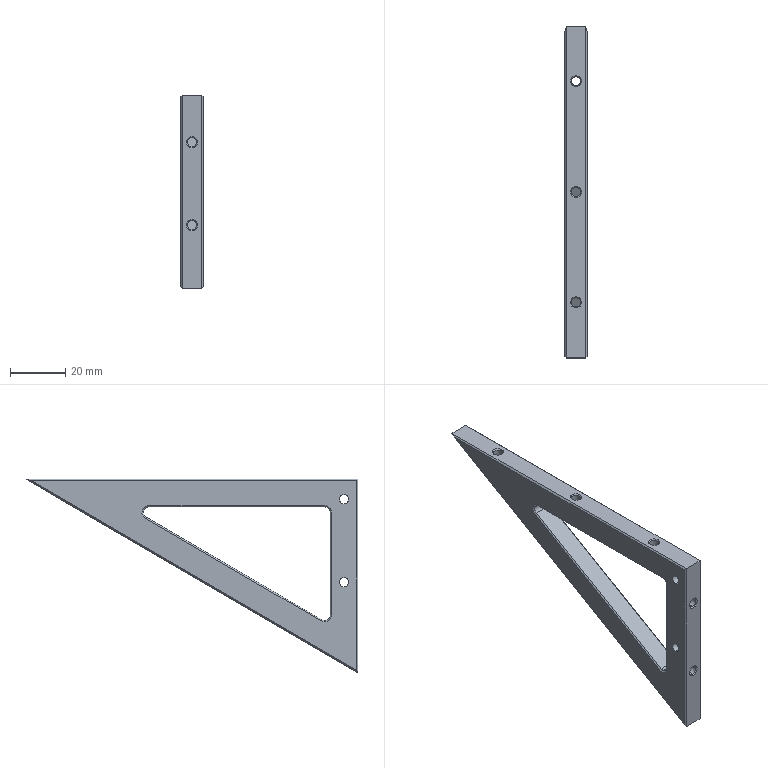Part | SolidWorks | features HoleWzd 3, Chamfer 1, Extrusion 1, Fillet 1 | 1 solid | 55 faces | box 8 x 120 x 70 mm | volume 20556 mm3 | plane 20 | cylinder 18 | cone 17 | commonest cylinder face diameters 3.3 x14 4 x4
STEP:
#1=CARTESIAN_POINT('',(0.,5.,-5.63));
#2=VERTEX_POINT('',#1);
#3=CARTESIAN_POINT('',(0.,5.,-8.93));
#4=VERTEX_POINT('',#3);
#5=CARTESIAN_POINT('',(0.,5.,-7.28));
#6=DIRECTION('',(1.,0.,0.));
#7=DIRECTION('',(0.,0.,-1.));
#8=AXIS2_PLACEMENT_3D('',#5,#6,#7);
#9=CIRCLE('',#8,1.65);
#10=EDGE_CURVE('',#2,#4,#9,.T.);
#11=ORIENTED_EDGE('',*,*,#10,.F.);
#12=CARTESIAN_POINT('',(8.,5.,-5.63));
#13=VERTEX_POINT('',#12);
#14=CARTESIAN_POINT('',(8.,5.,-5.63));
#15=DIRECTION('',(1.,0.,0.));
#16=VECTOR('',#15,1000.);
#17=LINE('',#14,#16);
#18=EDGE_CURVE('',#2,#13,#17,.T.);
#19=ORIENTED_EDGE('',*,*,#18,.T.);
#20=CARTESIAN_POINT('',(8.,5.,-8.93));
#21=VERTEX_POINT('',#20);
#22=CARTESIAN_POINT('',(8.,5.,-7.28));
#23=DIRECTION('',(1.,0.,0.));
#24=DIRECTION('',(0.,0.,-1.));
#25=AXIS2_PLACEMENT_3D('',#22,#23,#24);
#26=CIRCLE('',#25,1.65);
#27=EDGE_CURVE('',#13,#21,#26,.T.);
#28=ORIENTED_EDGE('',*,*,#27,.T.);
#29=CARTESIAN_POINT('',(8.,5.,-8.93));
#30=DIRECTION('',(1.,0.,0.));
#31=VECTOR('',#30,1000.);
#32=LINE('',#29,#31);
#33=EDGE_CURVE('',#4,#21,#32,.T.);
#34=ORIENTED_EDGE('',*,*,#33,.F.);
#35=EDGE_LOOP('',(#11,#19,#28,#34));
#36=FACE_OUTER_BOUND('',#35,.T.);
#37=CARTESIAN_POINT('',(8.,5.,-7.28));
#38=DIRECTION('',(1.,0.,0.));
#39=DIRECTION('',(0.,0.,-1.));
#40=AXIS2_PLACEMENT_3D('',#37,#38,#39);
#41=CYLINDRICAL_SURFACE('',#40,1.65);
#42=ADVANCED_FACE('',(#36),#41,.F.);
#43=CARTESIAN_POINT('',(0.,5.,-35.63));
#44=VERTEX_POINT('',#43);
#45=CARTESIAN_POINT('',(0.,5.,-38.93));
#46=VERTEX_POINT('',#45);
#47=CARTESIAN_POINT('',(0.,5.,-37.28));
#48=DIRECTION('',(1.,0.,0.));
#49=DIRECTION('',(0.,0.,-1.));
#50=AXIS2_PLACEMENT_3D('',#47,#48,#49);
#51=CIRCLE('',#50,1.65);
#52=EDGE_CURVE('',#44,#46,#51,.T.);
#53=ORIENTED_EDGE('',*,*,#52,.F.);
#54=CARTESIAN_POINT('',(8.,5.,-35.63));
#55=VERTEX_POINT('',#54);
#56=CARTESIAN_POINT('',(8.,5.,-35.63));
#57=DIRECTION('',(1.,0.,0.));
#58=VECTOR('',#57,1000.);
#59=LINE('',#56,#58);
#60=EDGE_CURVE('',#44,#55,#59,.T.);
#61=ORIENTED_EDGE('',*,*,#60,.T.);
#62=CARTESIAN_POINT('',(8.,5.,-38.93));
#63=VERTEX_POINT('',#62);
#64=CARTESIAN_POINT('',(8.,5.,-37.28));
#65=DIRECTION('',(1.,0.,0.));
#66=DIRECTION('',(0.,0.,-1.));
#67=AXIS2_PLACEMENT_3D('',#64,#65,#66);
#68=CIRCLE('',#67,1.65);
#69=EDGE_CURVE('',#55,#63,#68,.T.);
#70=ORIENTED_EDGE('',*,*,#69,.T.);
#71=CARTESIAN_POINT('',(8.,5.,-38.93));
#72=DIRECTION('',(1.,0.,0.));
#73=VECTOR('',#72,1000.);
#74=LINE('',#71,#73);
#75=EDGE_CURVE('',#46,#63,#74,.T.);
#76=ORIENTED_EDGE('',*,*,#75,.F.);
#77=EDGE_LOOP('',(#53,#61,#70,#76));
#78=FACE_OUTER_BOUND('',#77,.T.);
#79=CARTESIAN_POINT('',(8.,5.,-37.28));
#80=DIRECTION('',(1.,0.,0.));
#81=DIRECTION('',(0.,0.,-1.));
#82=AXIS2_PLACEMENT_3D('',#79,#80,#81);
#83=CYLINDRICAL_SURFACE('',#82,1.65);
#84=ADVANCED_FACE('',(#78),#83,.F.);
#85=CARTESIAN_POINT('',(7.5,12.,-51.108));
#86=VERTEX_POINT('',#85);
#87=CARTESIAN_POINT('',(7.5,13.008,-50.835));
#88=VERTEX_POINT('',#87);
#89=CARTESIAN_POINT('',(7.5,12.,-49.108));
#90=DIRECTION('',(1.,0.,0.));
#91=DIRECTION('',(0.,0.,1.));
#92=AXIS2_PLACEMENT_3D('',#89,#90,#91);
#93=CIRCLE('',#92,2.);
#94=EDGE_CURVE('',#86,#88,#93,.T.);
#95=ORIENTED_EDGE('',*,*,#94,.F.);
#96=CARTESIAN_POINT('',(8.,12.,-51.608));
#97=VERTEX_POINT('',#96);
#98=CARTESIAN_POINT('',(8.,12.,-51.608));
#99=DIRECTION('',(0.7071,0.,-0.7071));
#100=VECTOR('',#99,1000.);
#101=LINE('',#98,#100);
#102=EDGE_CURVE('',#86,#97,#101,.T.);
#103=ORIENTED_EDGE('',*,*,#102,.T.);
#104=CARTESIAN_POINT('',(8.,13.26,-51.267));
#105=VERTEX_POINT('',#104);
#106=CARTESIAN_POINT('',(8.,12.,-49.108));
#107=DIRECTION('',(-1.,0.,0.));
#108=DIRECTION('',(0.,0.,1.));
#109=AXIS2_PLACEMENT_3D('',#106,#107,#108);
#110=CIRCLE('',#109,2.5);
#111=EDGE_CURVE('',#105,#97,#110,.T.);
#112=ORIENTED_EDGE('',*,*,#111,.F.);
#113=CARTESIAN_POINT('',(7.5,13.008,-50.835));
#114=DIRECTION('',(0.7071,0.3563,-0.6108));
#115=VECTOR('',#114,1000.);
#116=LINE('',#113,#115);
#117=EDGE_CURVE('',#88,#105,#116,.T.);
#118=ORIENTED_EDGE('',*,*,#117,.F.);
#119=EDGE_LOOP('',(#95,#103,#112,#118));
#120=FACE_OUTER_BOUND('',#119,.T.);
#121=CARTESIAN_POINT('',(8.,12.,-49.108));
#122=DIRECTION('',(1.,0.,0.));
#123=DIRECTION('',(0.,0.,-1.));
#124=AXIS2_PLACEMENT_3D('',#121,#122,#123);
#125=CONICAL_SURFACE('',#124,2.5,0.7854);
#126=ADVANCED_FACE('',(#120),#125,.F.);
#127=CARTESIAN_POINT('',(0.5,13.008,-50.835));
#128=VERTEX_POINT('',#127);
#129=CARTESIAN_POINT('',(0.5,12.,-51.108));
#130=VERTEX_POINT('',#129);
#131=CARTESIAN_POINT('',(0.5,12.,-49.108));
#132=DIRECTION('',(-1.,0.,0.));
#133=DIRECTION('',(0.,0.,1.));
#134=AXIS2_PLACEMENT_3D('',#131,#132,#133);
#135=CIRCLE('',#134,2.);
#136=EDGE_CURVE('',#128,#130,#135,.T.);
#137=ORIENTED_EDGE('',*,*,#136,.T.);
#138=CARTESIAN_POINT('',(8.,12.,-51.108));
#139=DIRECTION('',(1.,0.,0.));
#140=VECTOR('',#139,1000.);
#141=LINE('',#138,#140);
#142=EDGE_CURVE('',#130,#86,#141,.T.);
#143=ORIENTED_EDGE('',*,*,#142,.T.);
#144=ORIENTED_EDGE('',*,*,#94,.T.);
#145=CARTESIAN_POINT('',(8.,13.008,-50.835));
#146=DIRECTION('',(1.,0.,0.));
#147=VECTOR('',#146,1000.);
#148=LINE('',#145,#147);
#149=EDGE_CURVE('',#128,#88,#148,.T.);
#150=ORIENTED_EDGE('',*,*,#149,.F.);
#151=EDGE_LOOP('',(#137,#143,#144,#150));
#152=FACE_OUTER_BOUND('',#151,.T.);
#153=CARTESIAN_POINT('',(8.,12.,-49.108));
#154=DIRECTION('',(1.,0.,0.));
#155=DIRECTION('',(0.,0.,-1.));
#156=AXIS2_PLACEMENT_3D('',#153,#154,#155);
#157=CYLINDRICAL_SURFACE('',#156,2.);
#158=ADVANCED_FACE('',(#152),#157,.F.);
#159=CARTESIAN_POINT('',(2.35,100.,-0.375));
#160=VERTEX_POINT('',#159);
#161=CARTESIAN_POINT('',(5.65,100.,-0.375));
#162=VERTEX_POINT('',#161);
#163=CARTESIAN_POINT('',(4.,100.,-0.375));
#164=DIRECTION('',(0.,0.,1.));
#165=DIRECTION('',(1.,0.,0.));
#166=AXIS2_PLACEMENT_3D('',#163,#164,#165);
#167=CIRCLE('',#166,1.65);
#168=EDGE_CURVE('',#160,#162,#167,.T.);
#169=ORIENTED_EDGE('',*,*,#168,.F.);
#170=CARTESIAN_POINT('',(1.975,100.,0.));
#171=VERTEX_POINT('',#170);
#172=CARTESIAN_POINT('',(1.975,100.,0.));
#173=DIRECTION('',(-0.7071,0.,0.7071));
#174=VECTOR('',#173,1000.);
#175=LINE('',#172,#174);
#176=EDGE_CURVE('',#160,#171,#175,.T.);
#177=ORIENTED_EDGE('',*,*,#176,.T.);
#178=CARTESIAN_POINT('',(6.025,100.,0.));
#179=VERTEX_POINT('',#178);
#180=CARTESIAN_POINT('',(4.,100.,0.));
#181=DIRECTION('',(0.,0.,1.));
#182=DIRECTION('',(1.,0.,0.));
#183=AXIS2_PLACEMENT_3D('',#180,#181,#182);
#184=CIRCLE('',#183,2.025);
#185=EDGE_CURVE('',#171,#179,#184,.T.);
#186=ORIENTED_EDGE('',*,*,#185,.T.);
#187=CARTESIAN_POINT('',(6.025,100.,0.));
#188=DIRECTION('',(0.7071,0.,0.7071));
#189=VECTOR('',#188,1000.);
#190=LINE('',#187,#189);
#191=EDGE_CURVE('',#162,#179,#190,.T.);
#192=ORIENTED_EDGE('',*,*,#191,.F.);
#193=EDGE_LOOP('',(#169,#177,#186,#192));
#194=FACE_OUTER_BOUND('',#193,.T.);
#195=CARTESIAN_POINT('',(4.,100.,0.));
#196=DIRECTION('',(0.,0.,1.));
#197=DIRECTION('',(1.,0.,0.));
#198=AXIS2_PLACEMENT_3D('',#195,#196,#197);
#199=CONICAL_SURFACE('',#198,2.025,0.7854);
#200=ADVANCED_FACE('',(#194),#199,.F.);
#201=CARTESIAN_POINT('',(2.35,100.,-11.667));
#202=VERTEX_POINT('',#201);
#203=CARTESIAN_POINT('',(5.65,100.,-11.667));
#204=VERTEX_POINT('',#203);
#205=CARTESIAN_POINT('',(2.35,100.,-11.667));
#206=CARTESIAN_POINT('',(2.35,96.7,-13.592));
#207=CARTESIAN_POINT('',(5.65,96.7,-13.592));
#208=CARTESIAN_POINT('',(5.65,100.,-11.667));
#209=(BOUNDED_CURVE()B_SPLINE_CURVE(3,(#205,#206,#207,#208),.UNSPECIFIED.,.F.,.F.)B_SPLINE_CURVE_WITH_KNOTS((4,4),(1.571,4.712),.UNSPECIFIED.)CURVE()GEOMETRIC_REPRESENTATION_ITEM()RATIONAL_B_SPLINE_CURVE((1.,0.3333,0.3333,1.))REPRESENTATION_ITEM(''));
#210=EDGE_CURVE('',#202,#204,#209,.T.);
#211=ORIENTED_EDGE('',*,*,#210,.F.);
#212=CARTESIAN_POINT('',(2.35,100.,0.));
#213=DIRECTION('',(0.,0.,1.));
#214=VECTOR('',#213,1000.);
#215=LINE('',#212,#214);
#216=EDGE_CURVE('',#202,#160,#215,.T.);
#217=ORIENTED_EDGE('',*,*,#216,.T.);
#218=ORIENTED_EDGE('',*,*,#168,.T.);
#219=CARTESIAN_POINT('',(5.65,100.,0.));
#220=DIRECTION('',(0.,0.,1.));
#221=VECTOR('',#220,1000.);
#222=LINE('',#219,#221);
#223=EDGE_CURVE('',#204,#162,#222,.T.);
#224=ORIENTED_EDGE('',*,*,#223,.F.);
#225=EDGE_LOOP('',(#211,#217,#218,#224));
#226=FACE_OUTER_BOUND('',#225,.T.);
#227=CARTESIAN_POINT('',(4.,100.,0.));
#228=DIRECTION('',(0.,0.,1.));
#229=DIRECTION('',(1.,0.,0.));
#230=AXIS2_PLACEMENT_3D('',#227,#228,#229);
#231=CYLINDRICAL_SURFACE('',#230,1.65);
#232=ADVANCED_FACE('',(#226),#231,.F.);
#233=CARTESIAN_POINT('',(2.35,60.,-0.375));
#234=VERTEX_POINT('',#233);
#235=CARTESIAN_POINT('',(5.65,60.,-0.375));
#236=VERTEX_POINT('',#235);
#237=CARTESIAN_POINT('',(4.,60.,-0.375));
#238=DIRECTION('',(0.,0.,1.));
#239=DIRECTION('',(1.,0.,0.));
#240=AXIS2_PLACEMENT_3D('',#237,#238,#239);
#241=CIRCLE('',#240,1.65);
#242=EDGE_CURVE('',#234,#236,#241,.T.);
#243=ORIENTED_EDGE('',*,*,#242,.F.);
#244=CARTESIAN_POINT('',(1.975,60.,0.));
#245=VERTEX_POINT('',#244);
#246=CARTESIAN_POINT('',(1.975,60.,0.));
#247=DIRECTION('',(-0.7071,0.,0.7071));
#248=VECTOR('',#247,1000.);
#249=LINE('',#246,#248);
#250=EDGE_CURVE('',#234,#245,#249,.T.);
#251=ORIENTED_EDGE('',*,*,#250,.T.);
#252=CARTESIAN_POINT('',(6.025,60.,0.));
#253=VERTEX_POINT('',#252);
#254=CARTESIAN_POINT('',(4.,60.,0.));
#255=DIRECTION('',(0.,0.,1.));
#256=DIRECTION('',(1.,0.,0.));
#257=AXIS2_PLACEMENT_3D('',#254,#255,#256);
#258=CIRCLE('',#257,2.025);
#259=EDGE_CURVE('',#245,#253,#258,.T.);
#260=ORIENTED_EDGE('',*,*,#259,.T.);
#261=CARTESIAN_POINT('',(6.025,60.,0.));
#262=DIRECTION('',(0.7071,0.,0.7071));
#263=VECTOR('',#262,1000.);
#264=LINE('',#261,#263);
#265=EDGE_CURVE('',#236,#253,#264,.T.);
#266=ORIENTED_EDGE('',*,*,#265,.F.);
#267=EDGE_LOOP('',(#243,#251,#260,#266));
#268=FACE_OUTER_BOUND('',#267,.T.);
#269=CARTESIAN_POINT('',(4.,60.,0.));
#270=DIRECTION('',(0.,0.,1.));
#271=DIRECTION('',(1.,0.,0.));
#272=AXIS2_PLACEMENT_3D('',#269,#270,#271);
#273=CONICAL_SURFACE('',#272,2.025,0.7854);
#274=ADVANCED_FACE('',(#268),#273,.F.);
#275=CARTESIAN_POINT('',(5.65,60.,-10.));
#276=VERTEX_POINT('',#275);
#277=CARTESIAN_POINT('',(2.35,60.,-10.));
#278=VERTEX_POINT('',#277);
#279=CARTESIAN_POINT('',(4.,60.,-10.));
#280=DIRECTION('',(0.,0.,-1.));
#281=DIRECTION('',(0.,1.,0.));
#282=AXIS2_PLACEMENT_3D('',#279,#280,#281);
#283=CIRCLE('',#282,1.65);
#284=EDGE_CURVE('',#276,#278,#283,.T.);
#285=ORIENTED_EDGE('',*,*,#284,.T.);
#286=CARTESIAN_POINT('',(2.35,60.,0.));
#287=DIRECTION('',(0.,0.,1.));
#288=VECTOR('',#287,1000.);
#289=LINE('',#286,#288);
#290=EDGE_CURVE('',#278,#234,#289,.T.);
#291=ORIENTED_EDGE('',*,*,#290,.T.);
#292=ORIENTED_EDGE('',*,*,#242,.T.);
#293=CARTESIAN_POINT('',(5.65,60.,0.));
#294=DIRECTION('',(0.,0.,1.));
#295=VECTOR('',#294,1000.);
#296=LINE('',#293,#295);
#297=EDGE_CURVE('',#276,#236,#296,.T.);
#298=ORIENTED_EDGE('',*,*,#297,.F.);
#299=EDGE_LOOP('',(#285,#291,#292,#298));
#300=FACE_OUTER_BOUND('',#299,.T.);
#301=CARTESIAN_POINT('',(4.,60.,0.));
#302=DIRECTION('',(0.,0.,1.));
#303=DIRECTION('',(1.,0.,0.));
#304=AXIS2_PLACEMENT_3D('',#301,#302,#303);
#305=CYLINDRICAL_SURFACE('',#304,1.65);
#306=ADVANCED_FACE('',(#300),#305,.F.);
#307=CARTESIAN_POINT('',(2.35,20.,-0.375));
#308=VERTEX_POINT('',#307);
#309=CARTESIAN_POINT('',(5.65,20.,-0.375));
#310=VERTEX_POINT('',#309);
#311=CARTESIAN_POINT('',(4.,20.,-0.375));
#312=DIRECTION('',(0.,0.,1.));
#313=DIRECTION('',(1.,0.,0.));
#314=AXIS2_PLACEMENT_3D('',#311,#312,#313);
#315=CIRCLE('',#314,1.65);
#316=EDGE_CURVE('',#308,#310,#315,.T.);
#317=ORIENTED_EDGE('',*,*,#316,.F.);
#318=CARTESIAN_POINT('',(1.975,20.,0.));
#319=VERTEX_POINT('',#318);
#320=CARTESIAN_POINT('',(1.975,20.,0.));
#321=DIRECTION('',(-0.7071,0.,0.7071));
#322=VECTOR('',#321,1000.);
#323=LINE('',#320,#322);
#324=EDGE_CURVE('',#308,#319,#323,.T.);
#325=ORIENTED_EDGE('',*,*,#324,.T.);
#326=CARTESIAN_POINT('',(6.025,20.,0.));
#327=VERTEX_POINT('',#326);
#328=CARTESIAN_POINT('',(4.,20.,0.));
#329=DIRECTION('',(0.,0.,1.));
#330=DIRECTION('',(1.,0.,0.));
#331=AXIS2_PLACEMENT_3D('',#328,#329,#330);
#332=CIRCLE('',#331,2.025);
#333=EDGE_CURVE('',#319,#327,#332,.T.);
#334=ORIENTED_EDGE('',*,*,#333,.T.);
#335=CARTESIAN_POINT('',(6.025,20.,0.));
#336=DIRECTION('',(0.7071,0.,0.7071));
#337=VECTOR('',#336,1000.);
#338=LINE('',#335,#337);
#339=EDGE_CURVE('',#310,#327,#338,.T.);
#340=ORIENTED_EDGE('',*,*,#339,.F.);
#341=EDGE_LOOP('',(#317,#325,#334,#340));
#342=FACE_OUTER_BOUND('',#341,.T.);
#343=CARTESIAN_POINT('',(4.,20.,0.));
#344=DIRECTION('',(0.,0.,1.));
#345=DIRECTION('',(1.,0.,0.));
#346=AXIS2_PLACEMENT_3D('',#343,#344,#345);
#347=CONICAL_SURFACE('',#346,2.025,0.7854);
#348=ADVANCED_FACE('',(#342),#347,.F.);
#349=CARTESIAN_POINT('',(5.65,20.,-10.));
#350=VERTEX_POINT('',#349);
#351=CARTESIAN_POINT('',(2.35,20.,-10.));
#352=VERTEX_POINT('',#351);
#353=CARTESIAN_POINT('',(4.,20.,-10.));
#354=DIRECTION('',(0.,0.,-1.));
#355=DIRECTION('',(0.,1.,0.));
#356=AXIS2_PLACEMENT_3D('',#353,#354,#355);
#357=CIRCLE('',#356,1.65);
#358=EDGE_CURVE('',#350,#352,#357,.T.);
#359=ORIENTED_EDGE('',*,*,#358,.T.);
#360=CARTESIAN_POINT('',(2.35,20.,0.));
#361=DIRECTION('',(0.,0.,1.));
#362=VECTOR('',#361,1000.);
#363=LINE('',#360,#362);
#364=EDGE_CURVE('',#352,#308,#363,.T.);
#365=ORIENTED_EDGE('',*,*,#364,.T.);
#366=ORIENTED_EDGE('',*,*,#316,.T.);
#367=CARTESIAN_POINT('',(5.65,20.,0.));
#368=DIRECTION('',(0.,0.,1.));
#369=VECTOR('',#368,1000.);
#370=LINE('',#367,#369);
#371=EDGE_CURVE('',#350,#310,#370,.T.);
#372=ORIENTED_EDGE('',*,*,#371,.F.);
#373=EDGE_LOOP('',(#359,#365,#366,#372));
#374=FACE_OUTER_BOUND('',#373,.T.);
#375=CARTESIAN_POINT('',(4.,20.,0.));
#376=DIRECTION('',(0.,0.,1.));
#377=DIRECTION('',(1.,0.,0.));
#378=AXIS2_PLACEMENT_3D('',#375,#376,#377);
#379=CYLINDRICAL_SURFACE('',#378,1.65);
#380=ADVANCED_FACE('',(#374),#379,.F.);
#381=CARTESIAN_POINT('',(4.,0.375,-45.35));
#382=VERTEX_POINT('',#381);
#383=CARTESIAN_POINT('',(4.,0.375,-48.65));
#384=VERTEX_POINT('',#383);
#385=CARTESIAN_POINT('',(4.,0.375,-47.));
#386=DIRECTION('',(0.,-1.,0.));
#387=DIRECTION('',(0.,0.,-1.));
#388=AXIS2_PLACEMENT_3D('',#385,#386,#387);
#389=CIRCLE('',#388,1.65);
#390=EDGE_CURVE('',#382,#384,#389,.T.);
#391=ORIENTED_EDGE('',*,*,#390,.F.);
#392=CARTESIAN_POINT('',(4.,0.,-44.975));
#393=VERTEX_POINT('',#392);
#394=CARTESIAN_POINT('',(4.,0.,-44.975));
#395=DIRECTION('',(0.,-0.7071,0.7071));
#396=VECTOR('',#395,1000.);
#397=LINE('',#394,#396);
#398=EDGE_CURVE('',#382,#393,#397,.T.);
#399=ORIENTED_EDGE('',*,*,#398,.T.);
#400=CARTESIAN_POINT('',(4.,0.,-49.025));
#401=VERTEX_POINT('',#400);
#402=CARTESIAN_POINT('',(4.,0.,-47.));
#403=DIRECTION('',(0.,-1.,0.));
#404=DIRECTION('',(0.,0.,-1.));
#405=AXIS2_PLACEMENT_3D('',#402,#403,#404);
#406=CIRCLE('',#405,2.025);
#407=EDGE_CURVE('',#393,#401,#406,.T.);
#408=ORIENTED_EDGE('',*,*,#407,.T.);
#409=CARTESIAN_POINT('',(4.,0.,-49.025));
#410=DIRECTION('',(0.,-0.7071,-0.7071));
#411=VECTOR('',#410,1000.);
#412=LINE('',#409,#411);
#413=EDGE_CURVE('',#384,#401,#412,.T.);
#414=ORIENTED_EDGE('',*,*,#413,.F.);
#415=EDGE_LOOP('',(#391,#399,#408,#414));
#416=FACE_OUTER_BOUND('',#415,.T.);
#417=CARTESIAN_POINT('',(4.,0.,-47.));
#418=DIRECTION('',(0.,-1.,0.));
#419=DIRECTION('',(0.,0.,-1.));
#420=AXIS2_PLACEMENT_3D('',#417,#418,#419);
#421=CONICAL_SURFACE('',#420,2.025,0.7854);
#422=ADVANCED_FACE('',(#416),#421,.F.);
#423=CARTESIAN_POINT('',(4.,10.,-48.65));
#424=VERTEX_POINT('',#423);
#425=CARTESIAN_POINT('',(4.,10.,-45.35));
#426=VERTEX_POINT('',#425);
#427=CARTESIAN_POINT('',(4.,10.,-47.));
#428=DIRECTION('',(0.,1.,0.));
#429=DIRECTION('',(0.,0.,1.));
#430=AXIS2_PLACEMENT_3D('',#427,#428,#429);
#431=CIRCLE('',#430,1.65);
#432=EDGE_CURVE('',#424,#426,#431,.T.);
#433=ORIENTED_EDGE('',*,*,#432,.T.);
#434=CARTESIAN_POINT('',(4.,0.,-45.35));
#435=DIRECTION('',(0.,-1.,0.));
#436=VECTOR('',#435,1000.);
#437=LINE('',#434,#436);
#438=EDGE_CURVE('',#426,#382,#437,.T.);
#439=ORIENTED_EDGE('',*,*,#438,.T.);
#440=ORIENTED_EDGE('',*,*,#390,.T.);
#441=CARTESIAN_POINT('',(4.,0.,-48.65));
#442=DIRECTION('',(0.,-1.,0.));
#443=VECTOR('',#442,1000.);
#444=LINE('',#441,#443);
#445=EDGE_CURVE('',#424,#384,#444,.T.);
#446=ORIENTED_EDGE('',*,*,#445,.F.);
#447=EDGE_LOOP('',(#433,#439,#440,#446));
#448=FACE_OUTER_BOUND('',#447,.T.);
#449=CARTESIAN_POINT('',(4.,0.,-47.));
#450=DIRECTION('',(0.,-1.,0.));
#451=DIRECTION('',(0.,0.,-1.));
#452=AXIS2_PLACEMENT_3D('',#449,#450,#451);
#453=CYLINDRICAL_SURFACE('',#452,1.65);
#454=ADVANCED_FACE('',(#448),#453,.F.);
#455=CARTESIAN_POINT('',(4.,0.375,-15.35));
#456=VERTEX_POINT('',#455);
#457=CARTESIAN_POINT('',(4.,0.375,-18.65));
#458=VERTEX_POINT('',#457);
#459=CARTESIAN_POINT('',(4.,0.375,-17.));
#460=DIRECTION('',(0.,-1.,0.));
#461=DIRECTION('',(0.,0.,-1.));
#462=AXIS2_PLACEMENT_3D('',#459,#460,#461);
#463=CIRCLE('',#462,1.65);
#464=EDGE_CURVE('',#456,#458,#463,.T.);
#465=ORIENTED_EDGE('',*,*,#464,.F.);
#466=CARTESIAN_POINT('',(4.,0.,-14.975));
#467=VERTEX_POINT('',#466);
#468=CARTESIAN_POINT('',(4.,0.,-14.975));
#469=DIRECTION('',(0.,-0.7071,0.7071));
#470=VECTOR('',#469,1000.);
#471=LINE('',#468,#470);
#472=EDGE_CURVE('',#456,#467,#471,.T.);
#473=ORIENTED_EDGE('',*,*,#472,.T.);
#474=CARTESIAN_POINT('',(4.,0.,-19.025));
#475=VERTEX_POINT('',#474);
#476=CARTESIAN_POINT('',(4.,0.,-17.));
#477=DIRECTION('',(0.,-1.,0.));
#478=DIRECTION('',(0.,0.,-1.));
#479=AXIS2_PLACEMENT_3D('',#476,#477,#478);
#480=CIRCLE('',#479,2.025);
#481=EDGE_CURVE('',#467,#475,#480,.T.);
#482=ORIENTED_EDGE('',*,*,#481,.T.);
#483=CARTESIAN_POINT('',(4.,0.,-19.025));
#484=DIRECTION('',(0.,-0.7071,-0.7071));
#485=VECTOR('',#484,1000.);
#486=LINE('',#483,#485);
#487=EDGE_CURVE('',#458,#475,#486,.T.);
#488=ORIENTED_EDGE('',*,*,#487,.F.);
#489=EDGE_LOOP('',(#465,#473,#482,#488));
#490=FACE_OUTER_BOUND('',#489,.T.);
#491=CARTESIAN_POINT('',(4.,0.,-17.));
#492=DIRECTION('',(0.,-1.,0.));
#493=DIRECTION('',(0.,0.,-1.));
#494=AXIS2_PLACEMENT_3D('',#491,#492,#493);
#495=CONICAL_SURFACE('',#494,2.025,0.7854);
#496=ADVANCED_FACE('',(#490),#495,.F.);
#497=CARTESIAN_POINT('',(4.,10.,-18.65));
#498=VERTEX_POINT('',#497);
#499=CARTESIAN_POINT('',(4.,10.,-15.35));
#500=VERTEX_POINT('',#499);
#501=CARTESIAN_POINT('',(4.,10.,-17.));
#502=DIRECTION('',(0.,1.,0.));
#503=DIRECTION('',(0.,0.,1.));
#504=AXIS2_PLACEMENT_3D('',#501,#502,#503);
#505=CIRCLE('',#504,1.65);
#506=EDGE_CURVE('',#498,#500,#505,.T.);
#507=ORIENTED_EDGE('',*,*,#506,.T.);
#508=CARTESIAN_POINT('',(4.,0.,-15.35));
#509=DIRECTION('',(0.,-1.,0.));
#510=VECTOR('',#509,1000.);
#511=LINE('',#508,#510);
#512=EDGE_CURVE('',#500,#456,#511,.T.);
#513=ORIENTED_EDGE('',*,*,#512,.T.);
#514=ORIENTED_EDGE('',*,*,#464,.T.);
#515=CARTESIAN_POINT('',(4.,0.,-18.65));
#516=DIRECTION('',(0.,-1.,0.));
#517=VECTOR('',#516,1000.);
#518=LINE('',#515,#517);
#519=EDGE_CURVE('',#498,#458,#518,.T.);
#520=ORIENTED_EDGE('',*,*,#519,.F.);
#521=EDGE_LOOP('',(#507,#513,#514,#520));
#522=FACE_OUTER_BOUND('',#521,.T.);
#523=CARTESIAN_POINT('',(4.,0.,-17.));
#524=DIRECTION('',(0.,-1.,0.));
#525=DIRECTION('',(0.,0.,-1.));
#526=AXIS2_PLACEMENT_3D('',#523,#524,#525);
#527=CYLINDRICAL_SURFACE('',#526,1.65);
#528=ADVANCED_FACE('',(#522),#527,.F.);
#529=CARTESIAN_POINT('',(4.,100.,0.));
#530=DIRECTION('',(0.,0.,1.));
#531=DIRECTION('',(1.,0.,0.));
#532=AXIS2_PLACEMENT_3D('',#529,#530,#531);
#533=CIRCLE('',#532,2.025);
#534=EDGE_CURVE('',#179,#171,#533,.T.);
#535=ORIENTED_EDGE('',*,*,#534,.F.);
#536=ORIENTED_EDGE('',*,*,#185,.F.);
#537=EDGE_LOOP('',(#535,#536));
#538=FACE_BOUND('',#537,.T.);
#539=CARTESIAN_POINT('',(4.,20.,0.));
#540=DIRECTION('',(0.,0.,1.));
#541=DIRECTION('',(1.,0.,0.));
#542=AXIS2_PLACEMENT_3D('',#539,#540,#541);
#543=CIRCLE('',#542,2.025);
#544=EDGE_CURVE('',#327,#319,#543,.T.);
#545=ORIENTED_EDGE('',*,*,#544,.F.);
#546=ORIENTED_EDGE('',*,*,#333,.F.);
#547=EDGE_LOOP('',(#545,#546));
#548=FACE_BOUND('',#547,.T.);
#549=CARTESIAN_POINT('',(7.5,120.,0.));
#550=VERTEX_POINT('',#549);
#551=CARTESIAN_POINT('',(0.5,120.,0.));
#552=VERTEX_POINT('',#551);
#553=CARTESIAN_POINT('',(8.,120.,0.));
#554=DIRECTION('',(-1.,0.,0.));
#555=VECTOR('',#554,1000.);
#556=LINE('',#553,#555);
#557=EDGE_CURVE('',#550,#552,#556,.T.);
#558=ORIENTED_EDGE('',*,*,#557,.T.);
#559=CARTESIAN_POINT('',(0.5,0.,0.));
#560=VERTEX_POINT('',#559);
#561=CARTESIAN_POINT('',(0.5,0.,0.));
#562=DIRECTION('',(0.,-1.,0.));
#563=VECTOR('',#562,1000.);
#564=LINE('',#561,#563);
#565=EDGE_CURVE('',#552,#560,#564,.T.);
#566=ORIENTED_EDGE('',*,*,#565,.T.);
#567=CARTESIAN_POINT('',(7.5,0.,0.));
#568=VERTEX_POINT('',#567);
#569=CARTESIAN_POINT('',(8.,0.,0.));
#570=DIRECTION('',(-1.,0.,0.));
#571=VECTOR('',#570,1000.);
#572=LINE('',#569,#571);
#573=EDGE_CURVE('',#568,#560,#572,.T.);
#574=ORIENTED_EDGE('',*,*,#573,.F.);
#575=CARTESIAN_POINT('',(7.5,120.,0.));
#576=DIRECTION('',(0.,1.,0.));
#577=VECTOR('',#576,1000.);
#578=LINE('',#575,#577);
#579=EDGE_CURVE('',#568,#550,#578,.T.);
#580=ORIENTED_EDGE('',*,*,#579,.T.);
#581=EDGE_LOOP('',(#558,#566,#574,#580));
#582=FACE_OUTER_BOUND('',#581,.T.);
#583=CARTESIAN_POINT('',(4.,60.,0.));
#584=DIRECTION('',(0.,0.,1.));
#585=DIRECTION('',(1.,0.,0.));
#586=AXIS2_PLACEMENT_3D('',#583,#584,#585);
#587=CIRCLE('',#586,2.025);
#588=EDGE_CURVE('',#253,#245,#587,.T.);
#589=ORIENTED_EDGE('',*,*,#588,.F.);
#590=ORIENTED_EDGE('',*,*,#259,.F.);
#591=EDGE_LOOP('',(#589,#590));
#592=FACE_BOUND('',#591,.T.);
#593=CARTESIAN_POINT('',(8.,120.,0.));
#594=DIRECTION('',(0.,0.,-1.));
#595=DIRECTION('',(-1.,0.,0.));
#596=AXIS2_PLACEMENT_3D('',#593,#594,#595);
#597=PLANE('',#596);
#598=ADVANCED_FACE('',(#538,#548,#582,#592),#597,.F.);
#599=ORIENTED_EDGE('',*,*,#573,.T.);
#600=CARTESIAN_POINT('',(0.5,0.,-70.));
#601=VERTEX_POINT('',#600);
#602=CARTESIAN_POINT('',(0.5,0.,-70.));
#603=DIRECTION('',(0.,0.,-1.));
#604=VECTOR('',#603,1000.);
#605=LINE('',#602,#604);
#606=EDGE_CURVE('',#560,#601,#605,.T.);
#607=ORIENTED_EDGE('',*,*,#606,.T.);
#608=CARTESIAN_POINT('',(7.5,0.,-70.));
#609=VERTEX_POINT('',#608);
#610=CARTESIAN_POINT('',(8.,0.,-70.));
#611=DIRECTION('',(-1.,0.,0.));
#612=VECTOR('',#611,1000.);
#613=LINE('',#610,#612);
#614=EDGE_CURVE('',#609,#601,#613,.T.);
#615=ORIENTED_EDGE('',*,*,#614,.F.);
#616=CARTESIAN_POINT('',(7.5,0.,0.));
#617=DIRECTION('',(0.,0.,1.));
#618=VECTOR('',#617,1000.);
#619=LINE('',#616,#618);
#620=EDGE_CURVE('',#609,#568,#619,.T.);
#621=ORIENTED_EDGE('',*,*,#620,.T.);
#622=EDGE_LOOP('',(#599,#607,#615,#621));
#623=FACE_OUTER_BOUND('',#622,.T.);
#624=CARTESIAN_POINT('',(4.,0.,-17.));
#625=DIRECTION('',(0.,-1.,0.));
#626=DIRECTION('',(0.,0.,-1.));
#627=AXIS2_PLACEMENT_3D('',#624,#625,#626);
#628=CIRCLE('',#627,2.025);
#629=EDGE_CURVE('',#475,#467,#628,.T.);
#630=ORIENTED_EDGE('',*,*,#629,.F.);
#631=ORIENTED_EDGE('',*,*,#481,.F.);
#632=EDGE_LOOP('',(#630,#631));
#633=FACE_BOUND('',#632,.T.);
#634=CARTESIAN_POINT('',(4.,0.,-47.));
#635=DIRECTION('',(0.,-1.,0.));
#636=DIRECTION('',(0.,0.,-1.));
#637=AXIS2_PLACEMENT_3D('',#634,#635,#636);
#638=CIRCLE('',#637,2.025);
#639=EDGE_CURVE('',#401,#393,#638,.T.);
#640=ORIENTED_EDGE('',*,*,#639,.F.);
#641=ORIENTED_EDGE('',*,*,#407,.F.);
#642=EDGE_LOOP('',(#640,#641));
#643=FACE_BOUND('',#642,.T.);
#644=CARTESIAN_POINT('',(8.,0.,0.));
#645=DIRECTION('',(0.,1.,0.));
#646=DIRECTION('',(0.,0.,1.));
#647=AXIS2_PLACEMENT_3D('',#644,#645,#646);
#648=PLANE('',#647);
#649=ADVANCED_FACE('',(#623,#633,#643),#648,.F.);
#650=CARTESIAN_POINT('',(8.,5.,-7.28));
#651=DIRECTION('',(1.,0.,0.));
#652=DIRECTION('',(0.,0.,-1.));
#653=AXIS2_PLACEMENT_3D('',#650,#651,#652);
#654=CIRCLE('',#653,1.65);
#655=EDGE_CURVE('',#21,#13,#654,.T.);
#656=ORIENTED_EDGE('',*,*,#655,.F.);
#657=ORIENTED_EDGE('',*,*,#27,.F.);
#658=EDGE_LOOP('',(#656,#657));
#659=FACE_BOUND('',#658,.T.);
#660=CARTESIAN_POINT('',(8.,5.,-37.28));
#661=DIRECTION('',(1.,0.,0.));
#662=DIRECTION('',(0.,0.,-1.));
#663=AXIS2_PLACEMENT_3D('',#660,#661,#662);
#664=CIRCLE('',#663,1.65);
#665=EDGE_CURVE('',#63,#55,#664,.T.);
#666=ORIENTED_EDGE('',*,*,#665,.F.);
#667=ORIENTED_EDGE('',*,*,#69,.F.);
#668=EDGE_LOOP('',(#666,#667));
#669=FACE_BOUND('',#668,.T.);
#670=CARTESIAN_POINT('',(8.,12.,-9.5));
#671=VERTEX_POINT('',#670);
#672=CARTESIAN_POINT('',(8.,75.613,-9.5));
#673=VERTEX_POINT('',#672);
#674=CARTESIAN_POINT('',(8.,75.613,-9.5));
#675=DIRECTION('',(0.,1.,0.));
#676=VECTOR('',#675,1000.);
#677=LINE('',#674,#676);
#678=EDGE_CURVE('',#671,#673,#677,.T.);
#679=ORIENTED_EDGE('',*,*,#678,.T.);
#680=CARTESIAN_POINT('',(8.,76.873,-14.159));
#681=VERTEX_POINT('',#680);
#682=CARTESIAN_POINT('',(8.,75.613,-12.));
#683=DIRECTION('',(-1.,0.,0.));
#684=DIRECTION('',(0.,0.,1.));
#685=AXIS2_PLACEMENT_3D('',#682,#683,#684);
#686=CIRCLE('',#685,2.5);
#687=EDGE_CURVE('',#673,#681,#686,.T.);
#688=ORIENTED_EDGE('',*,*,#687,.T.);
#689=CARTESIAN_POINT('',(8.,13.26,-51.267));
#690=DIRECTION('',(0.,-0.8638,-0.5039));
#691=VECTOR('',#690,1000.);
#692=LINE('',#689,#691);
#693=EDGE_CURVE('',#681,#105,#692,.T.);
#694=ORIENTED_EDGE('',*,*,#693,.T.);
#695=ORIENTED_EDGE('',*,*,#111,.T.);
#696=CARTESIAN_POINT('',(8.,9.5,-49.108));
#697=VERTEX_POINT('',#696);
#698=CARTESIAN_POINT('',(8.,12.,-49.108));
#699=DIRECTION('',(-1.,0.,0.));
#700=DIRECTION('',(0.,0.,1.));
#701=AXIS2_PLACEMENT_3D('',#698,#699,#700);
#702=CIRCLE('',#701,2.5);
#703=EDGE_CURVE('',#97,#697,#702,.T.);
#704=ORIENTED_EDGE('',*,*,#703,.T.);
#705=CARTESIAN_POINT('',(8.,9.5,-12.));
#706=VERTEX_POINT('',#705);
#707=CARTESIAN_POINT('',(8.,9.5,-12.));
#708=DIRECTION('',(0.,0.,1.));
#709=VECTOR('',#708,1000.);
#710=LINE('',#707,#709);
#711=EDGE_CURVE('',#697,#706,#710,.T.);
#712=ORIENTED_EDGE('',*,*,#711,.T.);
#713=CARTESIAN_POINT('',(8.,12.,-12.));
#714=DIRECTION('',(-1.,0.,0.));
#715=DIRECTION('',(0.,0.,1.));
#716=AXIS2_PLACEMENT_3D('',#713,#714,#715);
#717=CIRCLE('',#716,2.5);
#718=EDGE_CURVE('',#706,#671,#717,.T.);
#719=ORIENTED_EDGE('',*,*,#718,.T.);
#720=EDGE_LOOP('',(#679,#688,#694,#695,#704,#712,#719));
#721=FACE_BOUND('',#720,.T.);
#722=CARTESIAN_POINT('',(8.,118.151,-0.5));
#723=VERTEX_POINT('',#722);
#724=CARTESIAN_POINT('',(8.,0.5,-0.5));
#725=VERTEX_POINT('',#724);
#726=CARTESIAN_POINT('',(8.,0.,-0.5));
#727=DIRECTION('',(0.,-1.,0.));
#728=VECTOR('',#727,1000.);
#729=LINE('',#726,#728);
#730=EDGE_CURVE('',#723,#725,#729,.T.);
#731=ORIENTED_EDGE('',*,*,#730,.T.);
#732=CARTESIAN_POINT('',(8.,0.5,-69.129));
#733=VERTEX_POINT('',#732);
#734=CARTESIAN_POINT('',(8.,0.5,0.));
#735=DIRECTION('',(0.,0.,-1.));
#736=VECTOR('',#735,1000.);
#737=LINE('',#734,#736);
#738=EDGE_CURVE('',#725,#733,#737,.T.);
#739=ORIENTED_EDGE('',*,*,#738,.T.);
#740=CARTESIAN_POINT('',(8.,30.214,-51.796));
#741=DIRECTION('',(0.,0.8638,0.5039));
#742=VECTOR('',#741,1000.);
#743=LINE('',#740,#742);
#744=EDGE_CURVE('',#733,#723,#743,.T.);
#745=ORIENTED_EDGE('',*,*,#744,.T.);
#746=EDGE_LOOP('',(#731,#739,#745));
#747=FACE_OUTER_BOUND('',#746,.T.);
#748=CARTESIAN_POINT('',(8.,0.,0.));
#749=DIRECTION('',(-1.,0.,0.));
#750=DIRECTION('',(0.,0.,1.));
#751=AXIS2_PLACEMENT_3D('',#748,#749,#750);
#752=PLANE('',#751);
#753=ADVANCED_FACE('',(#659,#669,#721,#747),#752,.F.);
#754=CARTESIAN_POINT('',(0.,5.,-7.28));
#755=DIRECTION('',(1.,0.,0.));
#756=DIRECTION('',(0.,0.,-1.));
#757=AXIS2_PLACEMENT_3D('',#754,#755,#756);
#758=CIRCLE('',#757,1.65);
#759=EDGE_CURVE('',#4,#2,#758,.T.);
#760=ORIENTED_EDGE('',*,*,#759,.T.);
#761=ORIENTED_EDGE('',*,*,#10,.T.);
#762=EDGE_LOOP('',(#760,#761));
#763=FACE_BOUND('',#762,.T.);
#764=CARTESIAN_POINT('',(0.,5.,-37.28));
#765=DIRECTION('',(1.,0.,0.));
#766=DIRECTION('',(0.,0.,-1.));
#767=AXIS2_PLACEMENT_3D('',#764,#765,#766);
#768=CIRCLE('',#767,1.65);
#769=EDGE_CURVE('',#46,#44,#768,.T.);
#770=ORIENTED_EDGE('',*,*,#769,.T.);
#771=ORIENTED_EDGE('',*,*,#52,.T.);
#772=EDGE_LOOP('',(#770,#771));
#773=FACE_BOUND('',#772,.T.);
#774=CARTESIAN_POINT('',(0.,13.26,-51.267));
#775=VERTEX_POINT('',#774);
#776=CARTESIAN_POINT('',(0.,76.873,-14.159));
#777=VERTEX_POINT('',#776);
#778=CARTESIAN_POINT('',(0.,25.68,-44.022));
#779=DIRECTION('',(0.,0.8638,0.5039));
#780=VECTOR('',#779,1000.);
#781=LINE('',#778,#780);
#782=EDGE_CURVE('',#775,#777,#781,.T.);
#783=ORIENTED_EDGE('',*,*,#782,.T.);
#784=CARTESIAN_POINT('',(0.,75.613,-9.5));
#785=VERTEX_POINT('',#784);
#786=CARTESIAN_POINT('',(0.,75.613,-12.));
#787=DIRECTION('',(1.,0.,0.));
#788=DIRECTION('',(0.,0.,1.));
#789=AXIS2_PLACEMENT_3D('',#786,#787,#788);
#790=CIRCLE('',#789,2.5);
#791=EDGE_CURVE('',#777,#785,#790,.T.);
#792=ORIENTED_EDGE('',*,*,#791,.T.);
#793=CARTESIAN_POINT('',(0.,12.,-9.5));
#794=VERTEX_POINT('',#793);
#795=CARTESIAN_POINT('',(0.,0.,-9.5));
#796=DIRECTION('',(0.,-1.,0.));
#797=VECTOR('',#796,1000.);
#798=LINE('',#795,#797);
#799=EDGE_CURVE('',#785,#794,#798,.T.);
#800=ORIENTED_EDGE('',*,*,#799,.T.);
#801=CARTESIAN_POINT('',(0.,9.5,-12.));
#802=VERTEX_POINT('',#801);
#803=CARTESIAN_POINT('',(0.,12.,-12.));
#804=DIRECTION('',(1.,0.,0.));
#805=DIRECTION('',(0.,0.,1.));
#806=AXIS2_PLACEMENT_3D('',#803,#804,#805);
#807=CIRCLE('',#806,2.5);
#808=EDGE_CURVE('',#794,#802,#807,.T.);
#809=ORIENTED_EDGE('',*,*,#808,.T.);
#810=CARTESIAN_POINT('',(0.,9.5,-49.108));
#811=VERTEX_POINT('',#810);
#812=CARTESIAN_POINT('',(0.,9.5,0.));
#813=DIRECTION('',(0.,0.,-1.));
#814=VECTOR('',#813,1000.);
#815=LINE('',#812,#814);
#816=EDGE_CURVE('',#802,#811,#815,.T.);
#817=ORIENTED_EDGE('',*,*,#816,.T.);
#818=CARTESIAN_POINT('',(0.,12.,-49.108));
#819=DIRECTION('',(1.,0.,0.));
#820=DIRECTION('',(0.,0.,1.));
#821=AXIS2_PLACEMENT_3D('',#818,#819,#820);
#822=CIRCLE('',#821,2.5);
#823=EDGE_CURVE('',#811,#775,#822,.T.);
#824=ORIENTED_EDGE('',*,*,#823,.T.);
#825=EDGE_LOOP('',(#783,#792,#800,#809,#817,#824));
#826=FACE_BOUND('',#825,.T.);
#827=CARTESIAN_POINT('',(0.,0.5,-69.129));
#828=VERTEX_POINT('',#827);
#829=CARTESIAN_POINT('',(0.,0.5,-0.5));
#830=VERTEX_POINT('',#829);
#831=CARTESIAN_POINT('',(0.,0.5,0.));
#832=DIRECTION('',(0.,0.,1.));
#833=VECTOR('',#832,1000.);
#834=LINE('',#831,#833);
#835=EDGE_CURVE('',#828,#830,#834,.T.);
#836=ORIENTED_EDGE('',*,*,#835,.T.);
#837=CARTESIAN_POINT('',(0.,118.151,-0.5));
#838=VERTEX_POINT('',#837);
#839=CARTESIAN_POINT('',(0.,120.,-0.5));
#840=DIRECTION('',(0.,1.,0.));
#841=VECTOR('',#840,1000.);
#842=LINE('',#839,#841);
#843=EDGE_CURVE('',#830,#838,#842,.T.);
#844=ORIENTED_EDGE('',*,*,#843,.T.);
#845=CARTESIAN_POINT('',(0.,-0.2519,-69.568));
#846=DIRECTION('',(0.,-0.8638,-0.5039));
#847=VECTOR('',#846,1000.);
#848=LINE('',#845,#847);
#849=EDGE_CURVE('',#838,#828,#848,.T.);
#850=ORIENTED_EDGE('',*,*,#849,.T.);
#851=EDGE_LOOP('',(#836,#844,#850));
#852=FACE_OUTER_BOUND('',#851,.T.);
#853=CARTESIAN_POINT('',(0.,0.,0.));
#854=DIRECTION('',(-1.,0.,0.));
#855=DIRECTION('',(0.,0.,1.));
#856=AXIS2_PLACEMENT_3D('',#853,#854,#855);
#857=PLANE('',#856);
#858=ADVANCED_FACE('',(#763,#773,#826,#852),#857,.T.);
#859=CARTESIAN_POINT('',(5.65,100.,-11.667));
#860=CARTESIAN_POINT('',(5.65,103.3,-9.742));
#861=CARTESIAN_POINT('',(2.35,103.3,-9.742));
#862=CARTESIAN_POINT('',(2.35,100.,-11.667));
#863=(BOUNDED_CURVE()B_SPLINE_CURVE(3,(#859,#860,#861,#862),.UNSPECIFIED.,.F.,.F.)B_SPLINE_CURVE_WITH_KNOTS((4,4),(4.712,7.854),.UNSPECIFIED.)CURVE()GEOMETRIC_REPRESENTATION_ITEM()RATIONAL_B_SPLINE_CURVE((1.,0.3333,0.3333,1.))REPRESENTATION_ITEM(''));
#864=EDGE_CURVE('',#204,#202,#863,.T.);
#865=ORIENTED_EDGE('',*,*,#864,.T.);
#866=ORIENTED_EDGE('',*,*,#210,.T.);
#867=EDGE_LOOP('',(#865,#866));
#868=FACE_BOUND('',#867,.T.);
#869=ORIENTED_EDGE('',*,*,#614,.T.);
#870=CARTESIAN_POINT('',(0.5,120.,0.));
#871=DIRECTION('',(0.,0.8638,0.5039));
#872=VECTOR('',#871,1000.);
#873=LINE('',#870,#872);
#874=EDGE_CURVE('',#601,#552,#873,.T.);
#875=ORIENTED_EDGE('',*,*,#874,.T.);
#876=ORIENTED_EDGE('',*,*,#557,.F.);
#877=CARTESIAN_POINT('',(7.5,0.,-70.));
#878=DIRECTION('',(0.,-0.8638,-0.5039));
#879=VECTOR('',#878,1000.);
#880=LINE('',#877,#879);
#881=EDGE_CURVE('',#550,#609,#880,.T.);
#882=ORIENTED_EDGE('',*,*,#881,.T.);
#883=EDGE_LOOP('',(#869,#875,#876,#882));
#884=FACE_OUTER_BOUND('',#883,.T.);
#885=CARTESIAN_POINT('',(8.,0.,-70.));
#886=DIRECTION('',(0.,-0.5039,0.8638));
#887=DIRECTION('',(0.,-0.8638,-0.5039));
#888=AXIS2_PLACEMENT_3D('',#885,#886,#887);
#889=PLANE('',#888);
#890=ADVANCED_FACE('',(#868,#884),#889,.F.);
#891=CARTESIAN_POINT('',(7.5,76.621,-13.728));
#892=VERTEX_POINT('',#891);
#893=CARTESIAN_POINT('',(0.5,76.621,-13.728));
#894=VERTEX_POINT('',#893);
#895=CARTESIAN_POINT('',(0.,76.621,-13.728));
#896=DIRECTION('',(-1.,0.,0.));
#897=VECTOR('',#896,1000.);
#898=LINE('',#895,#897);
#899=EDGE_CURVE('',#892,#894,#898,.T.);
#900=ORIENTED_EDGE('',*,*,#899,.T.);
#901=CARTESIAN_POINT('',(0.5,10.,-52.59));
#902=DIRECTION('',(0.,-0.8638,-0.5039));
#903=VECTOR('',#902,1000.);
#904=LINE('',#901,#903);
#905=EDGE_CURVE('',#894,#128,#904,.T.);
#906=ORIENTED_EDGE('',*,*,#905,.T.);
#907=ORIENTED_EDGE('',*,*,#149,.T.);
#908=CARTESIAN_POINT('',(7.5,76.621,-13.728));
#909=DIRECTION('',(0.,0.8638,0.5039));
#910=VECTOR('',#909,1000.);
#911=LINE('',#908,#910);
#912=EDGE_CURVE('',#88,#892,#911,.T.);
#913=ORIENTED_EDGE('',*,*,#912,.T.);
#914=EDGE_LOOP('',(#900,#906,#907,#913));
#915=FACE_OUTER_BOUND('',#914,.T.);
#916=CARTESIAN_POINT('',(8.,10.,-52.59));
#917=DIRECTION('',(0.,-0.5039,0.8638));
#918=DIRECTION('',(0.,-0.8638,-0.5039));
#919=AXIS2_PLACEMENT_3D('',#916,#917,#918);
#920=PLANE('',#919);
#921=ADVANCED_FACE('',(#915),#920,.T.);
#922=ORIENTED_EDGE('',*,*,#284,.F.);
#923=CARTESIAN_POINT('',(4.,60.,-10.));
#924=DIRECTION('',(0.,0.,-1.));
#925=DIRECTION('',(0.,1.,0.));
#926=AXIS2_PLACEMENT_3D('',#923,#924,#925);
#927=CIRCLE('',#926,1.65);
#928=EDGE_CURVE('',#278,#276,#927,.T.);
#929=ORIENTED_EDGE('',*,*,#928,.F.);
#930=EDGE_LOOP('',(#922,#929));
#931=FACE_BOUND('',#930,.T.);
#932=ORIENTED_EDGE('',*,*,#358,.F.);
#933=CARTESIAN_POINT('',(4.,20.,-10.));
#934=DIRECTION('',(0.,0.,-1.));
#935=DIRECTION('',(0.,1.,0.));
#936=AXIS2_PLACEMENT_3D('',#933,#934,#935);
#937=CIRCLE('',#936,1.65);
#938=EDGE_CURVE('',#352,#350,#937,.T.);
#939=ORIENTED_EDGE('',*,*,#938,.F.);
#940=EDGE_LOOP('',(#932,#939));
#941=FACE_BOUND('',#940,.T.);
#942=CARTESIAN_POINT('',(7.5,12.,-10.));
#943=VERTEX_POINT('',#942);
#944=CARTESIAN_POINT('',(0.5,12.,-10.));
#945=VERTEX_POINT('',#944);
#946=CARTESIAN_POINT('',(0.,12.,-10.));
#947=DIRECTION('',(-1.,0.,0.));
#948=VECTOR('',#947,1000.);
#949=LINE('',#946,#948);
#950=EDGE_CURVE('',#943,#945,#949,.T.);
#951=ORIENTED_EDGE('',*,*,#950,.T.);
#952=CARTESIAN_POINT('',(0.5,75.613,-10.));
#953=VERTEX_POINT('',#952);
#954=CARTESIAN_POINT('',(0.5,83.011,-10.));
#955=DIRECTION('',(0.,1.,0.));
#956=VECTOR('',#955,1000.);
#957=LINE('',#954,#956);
#958=EDGE_CURVE('',#945,#953,#957,.T.);
#959=ORIENTED_EDGE('',*,*,#958,.T.);
#960=CARTESIAN_POINT('',(7.5,75.613,-10.));
#961=VERTEX_POINT('',#960);
#962=CARTESIAN_POINT('',(8.,75.613,-10.));
#963=DIRECTION('',(1.,0.,0.));
#964=VECTOR('',#963,1000.);
#965=LINE('',#962,#964);
#966=EDGE_CURVE('',#953,#961,#965,.T.);
#967=ORIENTED_EDGE('',*,*,#966,.T.);
#968=CARTESIAN_POINT('',(7.5,12.,-10.));
#969=DIRECTION('',(0.,-1.,0.));
#970=VECTOR('',#969,1000.);
#971=LINE('',#968,#970);
#972=EDGE_CURVE('',#961,#943,#971,.T.);
#973=ORIENTED_EDGE('',*,*,#972,.T.);
#974=EDGE_LOOP('',(#951,#959,#967,#973));
#975=FACE_OUTER_BOUND('',#974,.T.);
#976=CARTESIAN_POINT('',(8.,83.011,-10.));
#977=DIRECTION('',(0.,0.,-1.));
#978=DIRECTION('',(0.,1.,0.));
#979=AXIS2_PLACEMENT_3D('',#976,#977,#978);
#980=PLANE('',#979);
#981=ADVANCED_FACE('',(#931,#941,#975),#980,.T.);
#982=ORIENTED_EDGE('',*,*,#432,.F.);
#983=CARTESIAN_POINT('',(4.,10.,-47.));
#984=DIRECTION('',(0.,1.,0.));
#985=DIRECTION('',(0.,0.,1.));
#986=AXIS2_PLACEMENT_3D('',#983,#984,#985);
#987=CIRCLE('',#986,1.65);
#988=EDGE_CURVE('',#426,#424,#987,.T.);
#989=ORIENTED_EDGE('',*,*,#988,.F.);
#990=EDGE_LOOP('',(#982,#989));
#991=FACE_BOUND('',#990,.T.);
#992=ORIENTED_EDGE('',*,*,#506,.F.);
#993=CARTESIAN_POINT('',(4.,10.,-17.));
#994=DIRECTION('',(0.,1.,0.));
#995=DIRECTION('',(0.,0.,1.));
#996=AXIS2_PLACEMENT_3D('',#993,#994,#995);
#997=CIRCLE('',#996,1.65);
#998=EDGE_CURVE('',#500,#498,#997,.T.);
#999=ORIENTED_EDGE('',*,*,#998,.F.);
#1000=EDGE_LOOP('',(#992,#999));
#1001=FACE_BOUND('',#1000,.T.);
#1002=CARTESIAN_POINT('',(7.5,10.,-49.108));
#1003=VERTEX_POINT('',#1002);
#1004=CARTESIAN_POINT('',(0.5,10.,-49.108));
#1005=VERTEX_POINT('',#1004);
#1006=CARTESIAN_POINT('',(0.,10.,-49.108));
#1007=DIRECTION('',(-1.,0.,0.));
#1008=VECTOR('',#1007,1000.);
#1009=LINE('',#1006,#1008);
#1010=EDGE_CURVE('',#1003,#1005,#1009,.T.);
#1011=ORIENTED_EDGE('',*,*,#1010,.T.);
#1012=CARTESIAN_POINT('',(0.5,10.,-12.));
#1013=VERTEX_POINT('',#1012);
#1014=CARTESIAN_POINT('',(0.5,10.,-10.));
#1015=DIRECTION('',(0.,0.,1.));
#1016=VECTOR('',#1015,1000.);
#1017=LINE('',#1014,#1016);
#1018=EDGE_CURVE('',#1005,#1013,#1017,.T.);
#1019=ORIENTED_EDGE('',*,*,#1018,.T.);
#1020=CARTESIAN_POINT('',(7.5,10.,-12.));
#1021=VERTEX_POINT('',#1020);
#1022=CARTESIAN_POINT('',(8.,10.,-12.));
#1023=DIRECTION('',(1.,0.,0.));
#1024=VECTOR('',#1023,1000.);
#1025=LINE('',#1022,#1024);
#1026=EDGE_CURVE('',#1013,#1021,#1025,.T.);
#1027=ORIENTED_EDGE('',*,*,#1026,.T.);
#1028=CARTESIAN_POINT('',(7.5,10.,-49.108));
#1029=DIRECTION('',(0.,0.,-1.));
#1030=VECTOR('',#1029,1000.);
#1031=LINE('',#1028,#1030);
#1032=EDGE_CURVE('',#1021,#1003,#1031,.T.);
#1033=ORIENTED_EDGE('',*,*,#1032,.T.);
#1034=EDGE_LOOP('',(#1011,#1019,#1027,#1033));
#1035=FACE_OUTER_BOUND('',#1034,.T.);
#1036=CARTESIAN_POINT('',(8.,10.,-10.));
#1037=DIRECTION('',(0.,1.,0.));
#1038=DIRECTION('',(0.,0.,1.));
#1039=AXIS2_PLACEMENT_3D('',#1036,#1037,#1038);
#1040=PLANE('',#1039);
#1041=ADVANCED_FACE('',(#991,#1001,#1035),#1040,.T.);
#1042=ORIENTED_EDGE('',*,*,#512,.F.);
#1043=ORIENTED_EDGE('',*,*,#998,.T.);
#1044=ORIENTED_EDGE('',*,*,#519,.T.);
#1045=CARTESIAN_POINT('',(4.,0.375,-17.));
#1046=DIRECTION('',(0.,-1.,0.));
#1047=DIRECTION('',(0.,0.,-1.));
#1048=AXIS2_PLACEMENT_3D('',#1045,#1046,#1047);
#1049=CIRCLE('',#1048,1.65);
#1050=EDGE_CURVE('',#458,#456,#1049,.T.);
#1051=ORIENTED_EDGE('',*,*,#1050,.T.);
#1052=EDGE_LOOP('',(#1042,#1043,#1044,#1051));
#1053=FACE_OUTER_BOUND('',#1052,.T.);
#1054=CARTESIAN_POINT('',(4.,0.,-17.));
#1055=DIRECTION('',(0.,-1.,0.));
#1056=DIRECTION('',(0.,0.,-1.));
#1057=AXIS2_PLACEMENT_3D('',#1054,#1055,#1056);
#1058=CYLINDRICAL_SURFACE('',#1057,1.65);
#1059=ADVANCED_FACE('',(#1053),#1058,.F.);
#1060=ORIENTED_EDGE('',*,*,#472,.F.);
#1061=ORIENTED_EDGE('',*,*,#1050,.F.);
#1062=ORIENTED_EDGE('',*,*,#487,.T.);
#1063=ORIENTED_EDGE('',*,*,#629,.T.);
#1064=EDGE_LOOP('',(#1060,#1061,#1062,#1063));
#1065=FACE_OUTER_BOUND('',#1064,.T.);
#1066=CARTESIAN_POINT('',(4.,0.,-17.));
#1067=DIRECTION('',(0.,-1.,0.));
#1068=DIRECTION('',(0.,0.,-1.));
#1069=AXIS2_PLACEMENT_3D('',#1066,#1067,#1068);
#1070=CONICAL_SURFACE('',#1069,2.025,0.7854);
#1071=ADVANCED_FACE('',(#1065),#1070,.F.);
#1072=ORIENTED_EDGE('',*,*,#438,.F.);
#1073=ORIENTED_EDGE('',*,*,#988,.T.);
#1074=ORIENTED_EDGE('',*,*,#445,.T.);
#1075=CARTESIAN_POINT('',(4.,0.375,-47.));
#1076=DIRECTION('',(0.,-1.,0.));
#1077=DIRECTION('',(0.,0.,-1.));
#1078=AXIS2_PLACEMENT_3D('',#1075,#1076,#1077);
#1079=CIRCLE('',#1078,1.65);
#1080=EDGE_CURVE('',#384,#382,#1079,.T.);
#1081=ORIENTED_EDGE('',*,*,#1080,.T.);
#1082=EDGE_LOOP('',(#1072,#1073,#1074,#1081));
#1083=FACE_OUTER_BOUND('',#1082,.T.);
#1084=CARTESIAN_POINT('',(4.,0.,-47.));
#1085=DIRECTION('',(0.,-1.,0.));
#1086=DIRECTION('',(0.,0.,-1.));
#1087=AXIS2_PLACEMENT_3D('',#1084,#1085,#1086);
#1088=CYLINDRICAL_SURFACE('',#1087,1.65);
#1089=ADVANCED_FACE('',(#1083),#1088,.F.);
#1090=ORIENTED_EDGE('',*,*,#398,.F.);
#1091=ORIENTED_EDGE('',*,*,#1080,.F.);
#1092=ORIENTED_EDGE('',*,*,#413,.T.);
#1093=ORIENTED_EDGE('',*,*,#639,.T.);
#1094=EDGE_LOOP('',(#1090,#1091,#1092,#1093));
#1095=FACE_OUTER_BOUND('',#1094,.T.);
#1096=CARTESIAN_POINT('',(4.,0.,-47.));
#1097=DIRECTION('',(0.,-1.,0.));
#1098=DIRECTION('',(0.,0.,-1.));
#1099=AXIS2_PLACEMENT_3D('',#1096,#1097,#1098);
#1100=CONICAL_SURFACE('',#1099,2.025,0.7854);
#1101=ADVANCED_FACE('',(#1095),#1100,.F.);
#1102=ORIENTED_EDGE('',*,*,#364,.F.);
#1103=ORIENTED_EDGE('',*,*,#938,.T.);
#1104=ORIENTED_EDGE('',*,*,#371,.T.);
#1105=CARTESIAN_POINT('',(4.,20.,-0.375));
#1106=DIRECTION('',(0.,0.,1.));
#1107=DIRECTION('',(1.,0.,0.));
#1108=AXIS2_PLACEMENT_3D('',#1105,#1106,#1107);
#1109=CIRCLE('',#1108,1.65);
#1110=EDGE_CURVE('',#310,#308,#1109,.T.);
#1111=ORIENTED_EDGE('',*,*,#1110,.T.);
#1112=EDGE_LOOP('',(#1102,#1103,#1104,#1111));
#1113=FACE_OUTER_BOUND('',#1112,.T.);
#1114=CARTESIAN_POINT('',(4.,20.,0.));
#1115=DIRECTION('',(0.,0.,1.));
#1116=DIRECTION('',(1.,0.,0.));
#1117=AXIS2_PLACEMENT_3D('',#1114,#1115,#1116);
#1118=CYLINDRICAL_SURFACE('',#1117,1.65);
#1119=ADVANCED_FACE('',(#1113),#1118,.F.);
#1120=ORIENTED_EDGE('',*,*,#324,.F.);
#1121=ORIENTED_EDGE('',*,*,#1110,.F.);
#1122=ORIENTED_EDGE('',*,*,#339,.T.);
#1123=ORIENTED_EDGE('',*,*,#544,.T.);
#1124=EDGE_LOOP('',(#1120,#1121,#1122,#1123));
#1125=FACE_OUTER_BOUND('',#1124,.T.);
#1126=CARTESIAN_POINT('',(4.,20.,0.));
#1127=DIRECTION('',(0.,0.,1.));
#1128=DIRECTION('',(1.,0.,0.));
#1129=AXIS2_PLACEMENT_3D('',#1126,#1127,#1128);
#1130=CONICAL_SURFACE('',#1129,2.025,0.7854);
#1131=ADVANCED_FACE('',(#1125),#1130,.F.);
#1132=ORIENTED_EDGE('',*,*,#290,.F.);
#1133=ORIENTED_EDGE('',*,*,#928,.T.);
#1134=ORIENTED_EDGE('',*,*,#297,.T.);
#1135=CARTESIAN_POINT('',(4.,60.,-0.375));
#1136=DIRECTION('',(0.,0.,1.));
#1137=DIRECTION('',(1.,0.,0.));
#1138=AXIS2_PLACEMENT_3D('',#1135,#1136,#1137);
#1139=CIRCLE('',#1138,1.65);
#1140=EDGE_CURVE('',#236,#234,#1139,.T.);
#1141=ORIENTED_EDGE('',*,*,#1140,.T.);
#1142=EDGE_LOOP('',(#1132,#1133,#1134,#1141));
#1143=FACE_OUTER_BOUND('',#1142,.T.);
#1144=CARTESIAN_POINT('',(4.,60.,0.));
#1145=DIRECTION('',(0.,0.,1.));
#1146=DIRECTION('',(1.,0.,0.));
#1147=AXIS2_PLACEMENT_3D('',#1144,#1145,#1146);
#1148=CYLINDRICAL_SURFACE('',#1147,1.65);
#1149=ADVANCED_FACE('',(#1143),#1148,.F.);
#1150=ORIENTED_EDGE('',*,*,#250,.F.);
#1151=ORIENTED_EDGE('',*,*,#1140,.F.);
#1152=ORIENTED_EDGE('',*,*,#265,.T.);
#1153=ORIENTED_EDGE('',*,*,#588,.T.);
#1154=EDGE_LOOP('',(#1150,#1151,#1152,#1153));
#1155=FACE_OUTER_BOUND('',#1154,.T.);
#1156=CARTESIAN_POINT('',(4.,60.,0.));
#1157=DIRECTION('',(0.,0.,1.));
#1158=DIRECTION('',(1.,0.,0.));
#1159=AXIS2_PLACEMENT_3D('',#1156,#1157,#1158);
#1160=CONICAL_SURFACE('',#1159,2.025,0.7854);
#1161=ADVANCED_FACE('',(#1155),#1160,.F.);
#1162=ORIENTED_EDGE('',*,*,#216,.F.);
#1163=ORIENTED_EDGE('',*,*,#864,.F.);
#1164=ORIENTED_EDGE('',*,*,#223,.T.);
#1165=CARTESIAN_POINT('',(4.,100.,-0.375));
#1166=DIRECTION('',(0.,0.,1.));
#1167=DIRECTION('',(1.,0.,0.));
#1168=AXIS2_PLACEMENT_3D('',#1165,#1166,#1167);
#1169=CIRCLE('',#1168,1.65);
#1170=EDGE_CURVE('',#162,#160,#1169,.T.);
#1171=ORIENTED_EDGE('',*,*,#1170,.T.);
#1172=EDGE_LOOP('',(#1162,#1163,#1164,#1171));
#1173=FACE_OUTER_BOUND('',#1172,.T.);
#1174=CARTESIAN_POINT('',(4.,100.,0.));
#1175=DIRECTION('',(0.,0.,1.));
#1176=DIRECTION('',(1.,0.,0.));
#1177=AXIS2_PLACEMENT_3D('',#1174,#1175,#1176);
#1178=CYLINDRICAL_SURFACE('',#1177,1.65);
#1179=ADVANCED_FACE('',(#1173),#1178,.F.);
#1180=ORIENTED_EDGE('',*,*,#176,.F.);
#1181=ORIENTED_EDGE('',*,*,#1170,.F.);
#1182=ORIENTED_EDGE('',*,*,#191,.T.);
#1183=ORIENTED_EDGE('',*,*,#534,.T.);
#1184=EDGE_LOOP('',(#1180,#1181,#1182,#1183));
#1185=FACE_OUTER_BOUND('',#1184,.T.);
#1186=CARTESIAN_POINT('',(4.,100.,0.));
#1187=DIRECTION('',(0.,0.,1.));
#1188=DIRECTION('',(1.,0.,0.));
#1189=AXIS2_PLACEMENT_3D('',#1186,#1187,#1188);
#1190=CONICAL_SURFACE('',#1189,2.025,0.7854);
#1191=ADVANCED_FACE('',(#1185),#1190,.F.);
#1192=ORIENTED_EDGE('',*,*,#1026,.F.);
#1193=CARTESIAN_POINT('',(0.5,12.,-12.));
#1194=DIRECTION('',(-1.,0.,0.));
#1195=DIRECTION('',(0.,0.,1.));
#1196=AXIS2_PLACEMENT_3D('',#1193,#1194,#1195);
#1197=CIRCLE('',#1196,2.);
#1198=EDGE_CURVE('',#1013,#945,#1197,.T.);
#1199=ORIENTED_EDGE('',*,*,#1198,.T.);
#1200=ORIENTED_EDGE('',*,*,#950,.F.);
#1201=CARTESIAN_POINT('',(7.5,12.,-12.));
#1202=DIRECTION('',(1.,0.,0.));
#1203=DIRECTION('',(0.,0.,1.));
#1204=AXIS2_PLACEMENT_3D('',#1201,#1202,#1203);
#1205=CIRCLE('',#1204,2.);
#1206=EDGE_CURVE('',#943,#1021,#1205,.T.);
#1207=ORIENTED_EDGE('',*,*,#1206,.T.);
#1208=EDGE_LOOP('',(#1192,#1199,#1200,#1207));
#1209=FACE_OUTER_BOUND('',#1208,.T.);
#1210=CARTESIAN_POINT('',(8.,12.,-12.));
#1211=DIRECTION('',(1.,0.,0.));
#1212=DIRECTION('',(0.,0.,-1.));
#1213=AXIS2_PLACEMENT_3D('',#1210,#1211,#1212);
#1214=CYLINDRICAL_SURFACE('',#1213,2.);
#1215=ADVANCED_FACE('',(#1209),#1214,.F.);
#1216=ORIENTED_EDGE('',*,*,#142,.F.);
#1217=CARTESIAN_POINT('',(0.5,12.,-49.108));
#1218=DIRECTION('',(-1.,0.,0.));
#1219=DIRECTION('',(0.,0.,1.));
#1220=AXIS2_PLACEMENT_3D('',#1217,#1218,#1219);
#1221=CIRCLE('',#1220,2.);
#1222=EDGE_CURVE('',#130,#1005,#1221,.T.);
#1223=ORIENTED_EDGE('',*,*,#1222,.T.);
#1224=ORIENTED_EDGE('',*,*,#1010,.F.);
#1225=CARTESIAN_POINT('',(7.5,12.,-49.108));
#1226=DIRECTION('',(1.,0.,0.));
#1227=DIRECTION('',(0.,0.,1.));
#1228=AXIS2_PLACEMENT_3D('',#1225,#1226,#1227);
#1229=CIRCLE('',#1228,2.);
#1230=EDGE_CURVE('',#1003,#86,#1229,.T.);
#1231=ORIENTED_EDGE('',*,*,#1230,.T.);
#1232=EDGE_LOOP('',(#1216,#1223,#1224,#1231));
#1233=FACE_OUTER_BOUND('',#1232,.T.);
#1234=CARTESIAN_POINT('',(8.,12.,-49.108));
#1235=DIRECTION('',(1.,0.,0.));
#1236=DIRECTION('',(0.,0.,-1.));
#1237=AXIS2_PLACEMENT_3D('',#1234,#1235,#1236);
#1238=CYLINDRICAL_SURFACE('',#1237,2.);
#1239=ADVANCED_FACE('',(#1233),#1238,.F.);
#1240=ORIENTED_EDGE('',*,*,#966,.F.);
#1241=CARTESIAN_POINT('',(0.5,75.613,-12.));
#1242=DIRECTION('',(-1.,0.,0.));
#1243=DIRECTION('',(0.,0.,1.));
#1244=AXIS2_PLACEMENT_3D('',#1241,#1242,#1243);
#1245=CIRCLE('',#1244,2.);
#1246=EDGE_CURVE('',#953,#894,#1245,.T.);
#1247=ORIENTED_EDGE('',*,*,#1246,.T.);
#1248=ORIENTED_EDGE('',*,*,#899,.F.);
#1249=CARTESIAN_POINT('',(7.5,75.613,-12.));
#1250=DIRECTION('',(1.,0.,0.));
#1251=DIRECTION('',(0.,0.,1.));
#1252=AXIS2_PLACEMENT_3D('',#1249,#1250,#1251);
#1253=CIRCLE('',#1252,2.);
#1254=EDGE_CURVE('',#892,#961,#1253,.T.);
#1255=ORIENTED_EDGE('',*,*,#1254,.T.);
#1256=EDGE_LOOP('',(#1240,#1247,#1248,#1255));
#1257=FACE_OUTER_BOUND('',#1256,.T.);
#1258=CARTESIAN_POINT('',(8.,75.613,-12.));
#1259=DIRECTION('',(1.,0.,0.));
#1260=DIRECTION('',(0.,0.,-1.));
#1261=AXIS2_PLACEMENT_3D('',#1258,#1259,#1260);
#1262=CYLINDRICAL_SURFACE('',#1261,2.);
#1263=ADVANCED_FACE('',(#1257),#1262,.F.);
#1264=CARTESIAN_POINT('',(0.5,10.,-12.));
#1265=DIRECTION('',(-0.7071,-0.7071,0.));
#1266=VECTOR('',#1265,1000.);
#1267=LINE('',#1264,#1266);
#1268=EDGE_CURVE('',#1013,#802,#1267,.T.);
#1269=ORIENTED_EDGE('',*,*,#1268,.F.);
#1270=ORIENTED_EDGE('',*,*,#1018,.F.);
#1271=CARTESIAN_POINT('',(0.,9.5,-49.108));
#1272=DIRECTION('',(0.7071,0.7071,0.));
#1273=VECTOR('',#1272,1000.);
#1274=LINE('',#1271,#1273);
#1275=EDGE_CURVE('',#811,#1005,#1274,.T.);
#1276=ORIENTED_EDGE('',*,*,#1275,.F.);
#1277=ORIENTED_EDGE('',*,*,#816,.F.);
#1278=EDGE_LOOP('',(#1269,#1270,#1276,#1277));
#1279=FACE_OUTER_BOUND('',#1278,.T.);
#1280=CARTESIAN_POINT('',(0.,9.5,0.));
#1281=DIRECTION('',(0.7071,-0.7071,0.));
#1282=DIRECTION('',(0.,0.,-1.));
#1283=AXIS2_PLACEMENT_3D('',#1280,#1281,#1282);
#1284=PLANE('',#1283);
#1285=ADVANCED_FACE('',(#1279),#1284,.F.);
#1286=ORIENTED_EDGE('',*,*,#1275,.T.);
#1287=ORIENTED_EDGE('',*,*,#1222,.F.);
#1288=ORIENTED_EDGE('',*,*,#136,.F.);
#1289=CARTESIAN_POINT('',(0.,13.26,-51.267));
#1290=DIRECTION('',(0.7071,-0.3563,0.6108));
#1291=VECTOR('',#1290,1000.);
#1292=LINE('',#1289,#1291);
#1293=EDGE_CURVE('',#775,#128,#1292,.T.);
#1294=ORIENTED_EDGE('',*,*,#1293,.F.);
#1295=ORIENTED_EDGE('',*,*,#823,.F.);
#1296=EDGE_LOOP('',(#1286,#1287,#1288,#1294,#1295));
#1297=FACE_OUTER_BOUND('',#1296,.T.);
#1298=CARTESIAN_POINT('',(0.,12.,-49.108));
#1299=DIRECTION('',(-1.,0.,0.));
#1300=DIRECTION('',(0.,0.,1.));
#1301=AXIS2_PLACEMENT_3D('',#1298,#1299,#1300);
#1302=CONICAL_SURFACE('',#1301,2.5,0.7854);
#1303=ADVANCED_FACE('',(#1297),#1302,.F.);
#1304=ORIENTED_EDGE('',*,*,#1268,.T.);
#1305=ORIENTED_EDGE('',*,*,#808,.F.);
#1306=CARTESIAN_POINT('',(0.5,12.,-10.));
#1307=DIRECTION('',(-0.7071,0.,0.7071));
#1308=VECTOR('',#1307,1000.);
#1309=LINE('',#1306,#1308);
#1310=EDGE_CURVE('',#945,#794,#1309,.T.);
#1311=ORIENTED_EDGE('',*,*,#1310,.F.);
#1312=ORIENTED_EDGE('',*,*,#1198,.F.);
#1313=EDGE_LOOP('',(#1304,#1305,#1311,#1312));
#1314=FACE_OUTER_BOUND('',#1313,.T.);
#1315=CARTESIAN_POINT('',(0.,12.,-12.));
#1316=DIRECTION('',(-1.,0.,0.));
#1317=DIRECTION('',(0.,0.,1.));
#1318=AXIS2_PLACEMENT_3D('',#1315,#1316,#1317);
#1319=CONICAL_SURFACE('',#1318,2.5,0.7854);
#1320=ADVANCED_FACE('',(#1314),#1319,.F.);
#1321=ORIENTED_EDGE('',*,*,#1293,.T.);
#1322=ORIENTED_EDGE('',*,*,#905,.F.);
#1323=CARTESIAN_POINT('',(0.,76.873,-14.159));
#1324=DIRECTION('',(0.7071,-0.3563,0.6108));
#1325=VECTOR('',#1324,1000.);
#1326=LINE('',#1323,#1325);
#1327=EDGE_CURVE('',#777,#894,#1326,.T.);
#1328=ORIENTED_EDGE('',*,*,#1327,.F.);
#1329=ORIENTED_EDGE('',*,*,#782,.F.);
#1330=EDGE_LOOP('',(#1321,#1322,#1328,#1329));
#1331=FACE_OUTER_BOUND('',#1330,.T.);
#1332=CARTESIAN_POINT('',(0.,25.68,-44.022));
#1333=DIRECTION('',(0.7071,0.3563,-0.6108));
#1334=DIRECTION('',(0.,0.8638,0.5039));
#1335=AXIS2_PLACEMENT_3D('',#1332,#1333,#1334);
#1336=PLANE('',#1335);
#1337=ADVANCED_FACE('',(#1331),#1336,.F.);
#1338=ORIENTED_EDGE('',*,*,#1310,.T.);
#1339=ORIENTED_EDGE('',*,*,#799,.F.);
#1340=CARTESIAN_POINT('',(0.5,75.613,-10.));
#1341=DIRECTION('',(-0.7071,0.,0.7071));
#1342=VECTOR('',#1341,1000.);
#1343=LINE('',#1340,#1342);
#1344=EDGE_CURVE('',#953,#785,#1343,.T.);
#1345=ORIENTED_EDGE('',*,*,#1344,.F.);
#1346=ORIENTED_EDGE('',*,*,#958,.F.);
#1347=EDGE_LOOP('',(#1338,#1339,#1345,#1346));
#1348=FACE_OUTER_BOUND('',#1347,.T.);
#1349=CARTESIAN_POINT('',(0.,0.,-9.5));
#1350=DIRECTION('',(0.7071,0.,0.7071));
#1351=DIRECTION('',(0.,-1.,0.));
#1352=AXIS2_PLACEMENT_3D('',#1349,#1350,#1351);
#1353=PLANE('',#1352);
#1354=ADVANCED_FACE('',(#1348),#1353,.F.);
#1355=ORIENTED_EDGE('',*,*,#1327,.T.);
#1356=ORIENTED_EDGE('',*,*,#1246,.F.);
#1357=ORIENTED_EDGE('',*,*,#1344,.T.);
#1358=ORIENTED_EDGE('',*,*,#791,.F.);
#1359=EDGE_LOOP('',(#1355,#1356,#1357,#1358));
#1360=FACE_OUTER_BOUND('',#1359,.T.);
#1361=CARTESIAN_POINT('',(0.,75.613,-12.));
#1362=DIRECTION('',(-1.,0.,0.));
#1363=DIRECTION('',(0.,0.,1.));
#1364=AXIS2_PLACEMENT_3D('',#1361,#1362,#1363);
#1365=CONICAL_SURFACE('',#1364,2.5,0.7854);
#1366=ADVANCED_FACE('',(#1360),#1365,.F.);
#1367=CARTESIAN_POINT('',(-32.268,-1.207,-32.768));
#1368=DIRECTION('',(-0.2525,-0.9341,-0.2525));
#1369=VECTOR('',#1368,1000.);
#1370=LINE('',#1367,#1369);
#1371=EDGE_CURVE('',#552,#838,#1370,.T.);
#1372=ORIENTED_EDGE('',*,*,#1371,.F.);
#1373=ORIENTED_EDGE('',*,*,#874,.F.);
#1374=CARTESIAN_POINT('',(0.5,0.,-70.));
#1375=DIRECTION('',(0.4458,-0.4458,-0.7762));
#1376=VECTOR('',#1375,1000.);
#1377=LINE('',#1374,#1376);
#1378=EDGE_CURVE('',#828,#601,#1377,.T.);
#1379=ORIENTED_EDGE('',*,*,#1378,.F.);
#1380=ORIENTED_EDGE('',*,*,#849,.F.);
#1381=EDGE_LOOP('',(#1372,#1373,#1379,#1380));
#1382=FACE_OUTER_BOUND('',#1381,.T.);
#1383=CARTESIAN_POINT('',(0.5,0.,-70.));
#1384=DIRECTION('',(-0.7071,0.3563,-0.6108));
#1385=DIRECTION('',(0.,-0.8638,-0.5039));
#1386=AXIS2_PLACEMENT_3D('',#1383,#1384,#1385);
#1387=PLANE('',#1386);
#1388=ADVANCED_FACE('',(#1382),#1387,.T.);
#1389=ORIENTED_EDGE('',*,*,#1378,.T.);
#1390=ORIENTED_EDGE('',*,*,#606,.F.);
#1391=CARTESIAN_POINT('',(0.5,0.,0.));
#1392=DIRECTION('',(0.5774,-0.5774,0.5774));
#1393=VECTOR('',#1392,1000.);
#1394=LINE('',#1391,#1393);
#1395=EDGE_CURVE('',#830,#560,#1394,.T.);
#1396=ORIENTED_EDGE('',*,*,#1395,.F.);
#1397=ORIENTED_EDGE('',*,*,#835,.F.);
#1398=EDGE_LOOP('',(#1389,#1390,#1396,#1397));
#1399=FACE_OUTER_BOUND('',#1398,.T.);
#1400=CARTESIAN_POINT('',(0.5,0.,0.));
#1401=DIRECTION('',(-0.7071,-0.7071,0.));
#1402=DIRECTION('',(0.,0.,1.));
#1403=AXIS2_PLACEMENT_3D('',#1400,#1401,#1402);
#1404=PLANE('',#1403);
#1405=ADVANCED_FACE('',(#1399),#1404,.T.);
#1406=ORIENTED_EDGE('',*,*,#1371,.T.);
#1407=ORIENTED_EDGE('',*,*,#843,.F.);
#1408=ORIENTED_EDGE('',*,*,#1395,.T.);
#1409=ORIENTED_EDGE('',*,*,#565,.F.);
#1410=EDGE_LOOP('',(#1406,#1407,#1408,#1409));
#1411=FACE_OUTER_BOUND('',#1410,.T.);
#1412=CARTESIAN_POINT('',(0.5,120.,0.));
#1413=DIRECTION('',(-0.7071,0.,0.7071));
#1414=DIRECTION('',(0.,1.,0.));
#1415=AXIS2_PLACEMENT_3D('',#1412,#1413,#1414);
#1416=PLANE('',#1415);
#1417=ADVANCED_FACE('',(#1411),#1416,.T.);
#1418=CARTESIAN_POINT('',(7.5,10.,-49.108));
#1419=DIRECTION('',(0.7071,-0.7071,0.));
#1420=VECTOR('',#1419,1000.);
#1421=LINE('',#1418,#1420);
#1422=EDGE_CURVE('',#1003,#697,#1421,.T.);
#1423=ORIENTED_EDGE('',*,*,#1422,.F.);
#1424=ORIENTED_EDGE('',*,*,#1032,.F.);
#1425=CARTESIAN_POINT('',(8.,9.5,-12.));
#1426=DIRECTION('',(-0.7071,0.7071,0.));
#1427=VECTOR('',#1426,1000.);
#1428=LINE('',#1425,#1427);
#1429=EDGE_CURVE('',#706,#1021,#1428,.T.);
#1430=ORIENTED_EDGE('',*,*,#1429,.F.);
#1431=ORIENTED_EDGE('',*,*,#711,.F.);
#1432=EDGE_LOOP('',(#1423,#1424,#1430,#1431));
#1433=FACE_OUTER_BOUND('',#1432,.T.);
#1434=CARTESIAN_POINT('',(7.5,10.,-10.));
#1435=DIRECTION('',(0.7071,0.7071,0.));
#1436=DIRECTION('',(0.,0.,1.));
#1437=AXIS2_PLACEMENT_3D('',#1434,#1435,#1436);
#1438=PLANE('',#1437);
#1439=ADVANCED_FACE('',(#1433),#1438,.T.);
#1440=ORIENTED_EDGE('',*,*,#1429,.T.);
#1441=ORIENTED_EDGE('',*,*,#1206,.F.);
#1442=CARTESIAN_POINT('',(8.,12.,-9.5));
#1443=DIRECTION('',(-0.7071,0.,-0.7071));
#1444=VECTOR('',#1443,1000.);
#1445=LINE('',#1442,#1444);
#1446=EDGE_CURVE('',#671,#943,#1445,.T.);
#1447=ORIENTED_EDGE('',*,*,#1446,.F.);
#1448=ORIENTED_EDGE('',*,*,#718,.F.);
#1449=EDGE_LOOP('',(#1440,#1441,#1447,#1448));
#1450=FACE_OUTER_BOUND('',#1449,.T.);
#1451=CARTESIAN_POINT('',(8.,12.,-12.));
#1452=DIRECTION('',(1.,0.,0.));
#1453=DIRECTION('',(0.,0.,-1.));
#1454=AXIS2_PLACEMENT_3D('',#1451,#1452,#1453);
#1455=CONICAL_SURFACE('',#1454,2.5,0.7854);
#1456=ADVANCED_FACE('',(#1450),#1455,.F.);
#1457=ORIENTED_EDGE('',*,*,#102,.F.);
#1458=ORIENTED_EDGE('',*,*,#1230,.F.);
#1459=ORIENTED_EDGE('',*,*,#1422,.T.);
#1460=ORIENTED_EDGE('',*,*,#703,.F.);
#1461=EDGE_LOOP('',(#1457,#1458,#1459,#1460));
#1462=FACE_OUTER_BOUND('',#1461,.T.);
#1463=CARTESIAN_POINT('',(8.,12.,-49.108));
#1464=DIRECTION('',(1.,0.,0.));
#1465=DIRECTION('',(0.,0.,-1.));
#1466=AXIS2_PLACEMENT_3D('',#1463,#1464,#1465);
#1467=CONICAL_SURFACE('',#1466,2.5,0.7854);
#1468=ADVANCED_FACE('',(#1462),#1467,.F.);
#1469=ORIENTED_EDGE('',*,*,#1446,.T.);
#1470=ORIENTED_EDGE('',*,*,#972,.F.);
#1471=CARTESIAN_POINT('',(8.,75.613,-9.5));
#1472=DIRECTION('',(-0.7071,0.,-0.7071));
#1473=VECTOR('',#1472,1000.);
#1474=LINE('',#1471,#1473);
#1475=EDGE_CURVE('',#673,#961,#1474,.T.);
#1476=ORIENTED_EDGE('',*,*,#1475,.F.);
#1477=ORIENTED_EDGE('',*,*,#678,.F.);
#1478=EDGE_LOOP('',(#1469,#1470,#1476,#1477));
#1479=FACE_OUTER_BOUND('',#1478,.T.);
#1480=CARTESIAN_POINT('',(7.5,83.011,-10.));
#1481=DIRECTION('',(0.7071,0.,-0.7071));
#1482=DIRECTION('',(0.,1.,0.));
#1483=AXIS2_PLACEMENT_3D('',#1480,#1481,#1482);
#1484=PLANE('',#1483);
#1485=ADVANCED_FACE('',(#1479),#1484,.T.);
#1486=ORIENTED_EDGE('',*,*,#117,.T.);
#1487=ORIENTED_EDGE('',*,*,#693,.F.);
#1488=CARTESIAN_POINT('',(7.5,76.621,-13.728));
#1489=DIRECTION('',(0.7071,0.3563,-0.6108));
#1490=VECTOR('',#1489,1000.);
#1491=LINE('',#1488,#1490);
#1492=EDGE_CURVE('',#892,#681,#1491,.T.);
#1493=ORIENTED_EDGE('',*,*,#1492,.F.);
#1494=ORIENTED_EDGE('',*,*,#912,.F.);
#1495=EDGE_LOOP('',(#1486,#1487,#1493,#1494));
#1496=FACE_OUTER_BOUND('',#1495,.T.);
#1497=CARTESIAN_POINT('',(7.5,10.,-52.59));
#1498=DIRECTION('',(0.7071,-0.3563,0.6108));
#1499=DIRECTION('',(0.,-0.8638,-0.5039));
#1500=AXIS2_PLACEMENT_3D('',#1497,#1498,#1499);
#1501=PLANE('',#1500);
#1502=ADVANCED_FACE('',(#1496),#1501,.T.);
#1503=ORIENTED_EDGE('',*,*,#1475,.T.);
#1504=ORIENTED_EDGE('',*,*,#1254,.F.);
#1505=ORIENTED_EDGE('',*,*,#1492,.T.);
#1506=ORIENTED_EDGE('',*,*,#687,.F.);
#1507=EDGE_LOOP('',(#1503,#1504,#1505,#1506));
#1508=FACE_OUTER_BOUND('',#1507,.T.);
#1509=CARTESIAN_POINT('',(8.,75.613,-12.));
#1510=DIRECTION('',(1.,0.,0.));
#1511=DIRECTION('',(0.,0.,-1.));
#1512=AXIS2_PLACEMENT_3D('',#1509,#1510,#1511);
#1513=CONICAL_SURFACE('',#1512,2.5,0.7854);
#1514=ADVANCED_FACE('',(#1508),#1513,.F.);
#1515=CARTESIAN_POINT('',(7.833,0.3333,-0.3333));
#1516=DIRECTION('',(-0.5774,-0.5774,0.5774));
#1517=VECTOR('',#1516,1000.);
#1518=LINE('',#1515,#1517);
#1519=EDGE_CURVE('',#725,#568,#1518,.T.);
#1520=ORIENTED_EDGE('',*,*,#1519,.F.);
#1521=ORIENTED_EDGE('',*,*,#730,.F.);
#1522=CARTESIAN_POINT('',(32.013,29.33,-24.513));
#1523=DIRECTION('',(0.2525,-0.9341,-0.2525));
#1524=VECTOR('',#1523,1000.);
#1525=LINE('',#1522,#1524);
#1526=EDGE_CURVE('',#550,#723,#1525,.T.);
#1527=ORIENTED_EDGE('',*,*,#1526,.F.);
#1528=ORIENTED_EDGE('',*,*,#579,.F.);
#1529=EDGE_LOOP('',(#1520,#1521,#1527,#1528));
#1530=FACE_OUTER_BOUND('',#1529,.T.);
#1531=CARTESIAN_POINT('',(8.,0.,-0.5));
#1532=DIRECTION('',(-0.7071,0.,-0.7071));
#1533=DIRECTION('',(0.,-1.,0.));
#1534=AXIS2_PLACEMENT_3D('',#1531,#1532,#1533);
#1535=PLANE('',#1534);
#1536=ADVANCED_FACE('',(#1530),#1535,.F.);
#1537=ORIENTED_EDGE('',*,*,#1526,.T.);
#1538=ORIENTED_EDGE('',*,*,#744,.F.);
#1539=CARTESIAN_POINT('',(19.904,12.404,-48.404));
#1540=DIRECTION('',(0.4458,0.4458,0.7762));
#1541=VECTOR('',#1540,1000.);
#1542=LINE('',#1539,#1541);
#1543=EDGE_CURVE('',#609,#733,#1542,.T.);
#1544=ORIENTED_EDGE('',*,*,#1543,.F.);
#1545=ORIENTED_EDGE('',*,*,#881,.F.);
#1546=EDGE_LOOP('',(#1537,#1538,#1544,#1545));
#1547=FACE_OUTER_BOUND('',#1546,.T.);
#1548=CARTESIAN_POINT('',(8.,30.214,-51.796));
#1549=DIRECTION('',(-0.7071,-0.3563,0.6108));
#1550=DIRECTION('',(0.,0.8638,0.5039));
#1551=AXIS2_PLACEMENT_3D('',#1548,#1549,#1550);
#1552=PLANE('',#1551);
#1553=ADVANCED_FACE('',(#1547),#1552,.F.);
#1554=ORIENTED_EDGE('',*,*,#1519,.T.);
#1555=ORIENTED_EDGE('',*,*,#620,.F.);
#1556=ORIENTED_EDGE('',*,*,#1543,.T.);
#1557=ORIENTED_EDGE('',*,*,#738,.F.);
#1558=EDGE_LOOP('',(#1554,#1555,#1556,#1557));
#1559=FACE_OUTER_BOUND('',#1558,.T.);
#1560=CARTESIAN_POINT('',(8.,0.5,0.));
#1561=DIRECTION('',(-0.7071,0.7071,0.));
#1562=DIRECTION('',(0.,0.,-1.));
#1563=AXIS2_PLACEMENT_3D('',#1560,#1561,#1562);
#1564=PLANE('',#1563);
#1565=ADVANCED_FACE('',(#1559),#1564,.F.);
#1566=ORIENTED_EDGE('',*,*,#60,.F.);
#1567=ORIENTED_EDGE('',*,*,#769,.F.);
#1568=ORIENTED_EDGE('',*,*,#75,.T.);
#1569=ORIENTED_EDGE('',*,*,#665,.T.);
#1570=EDGE_LOOP('',(#1566,#1567,#1568,#1569));
#1571=FACE_OUTER_BOUND('',#1570,.T.);
#1572=CARTESIAN_POINT('',(8.,5.,-37.28));
#1573=DIRECTION('',(1.,0.,0.));
#1574=DIRECTION('',(0.,0.,-1.));
#1575=AXIS2_PLACEMENT_3D('',#1572,#1573,#1574);
#1576=CYLINDRICAL_SURFACE('',#1575,1.65);
#1577=ADVANCED_FACE('',(#1571),#1576,.F.);
#1578=ORIENTED_EDGE('',*,*,#18,.F.);
#1579=ORIENTED_EDGE('',*,*,#759,.F.);
#1580=ORIENTED_EDGE('',*,*,#33,.T.);
#1581=ORIENTED_EDGE('',*,*,#655,.T.);
#1582=EDGE_LOOP('',(#1578,#1579,#1580,#1581));
#1583=FACE_OUTER_BOUND('',#1582,.T.);
#1584=CARTESIAN_POINT('',(8.,5.,-7.28));
#1585=DIRECTION('',(1.,0.,0.));
#1586=DIRECTION('',(0.,0.,-1.));
#1587=AXIS2_PLACEMENT_3D('',#1584,#1585,#1586);
#1588=CYLINDRICAL_SURFACE('',#1587,1.65);
#1589=ADVANCED_FACE('',(#1583),#1588,.F.);
#1590=CLOSED_SHELL('',(#42,#84,#126,#158,#200,#232,#274,#306,#348,#380,#422,#454,#496,#528,#598,#649,#753,#858,#890,#921,#981,#1041,#1059,#1071,#1089,#1101,#1119,#1131,#1149,#1161,#1179,#1191,#1215,#1239,#1263,#1285,#1303,#1320,#1337,#1354,#1366,#1388,#1405,#1417,#1439,#1456,#1468,#1485,#1502,#1514,#1536,#1553,#1565,#1577,#1589));
#1591=MANIFOLD_SOLID_BREP('',#1590);
#1592=CARTESIAN_POINT('',(0.,0.,0.));
#1593=DIRECTION('',(0.,0.,1.));
#1594=DIRECTION('',(1.,0.,0.));
#1595=AXIS2_PLACEMENT_3D('',#1592,#1593,#1594);
#1596=(LENGTH_UNIT()NAMED_UNIT(*)SI_UNIT(.MILLI.,.METRE.));
#1597=UNCERTAINTY_MEASURE_WITH_UNIT(LENGTH_MEASURE(0.00001),#1596,'','');
#1598=(NAMED_UNIT(*)PLANE_ANGLE_UNIT()SI_UNIT($,.RADIAN.));
#1599=(NAMED_UNIT(*)SI_UNIT($,.STERADIAN.)SOLID_ANGLE_UNIT());
#1600=(GEOMETRIC_REPRESENTATION_CONTEXT(3)GLOBAL_UNCERTAINTY_ASSIGNED_CONTEXT((#1597))GLOBAL_UNIT_ASSIGNED_CONTEXT((#1596,#1598,#1599))REPRESENTATION_CONTEXT('',''));
#1601=ADVANCED_BREP_SHAPE_REPRESENTATION('',(#1591,#1595),#1600);